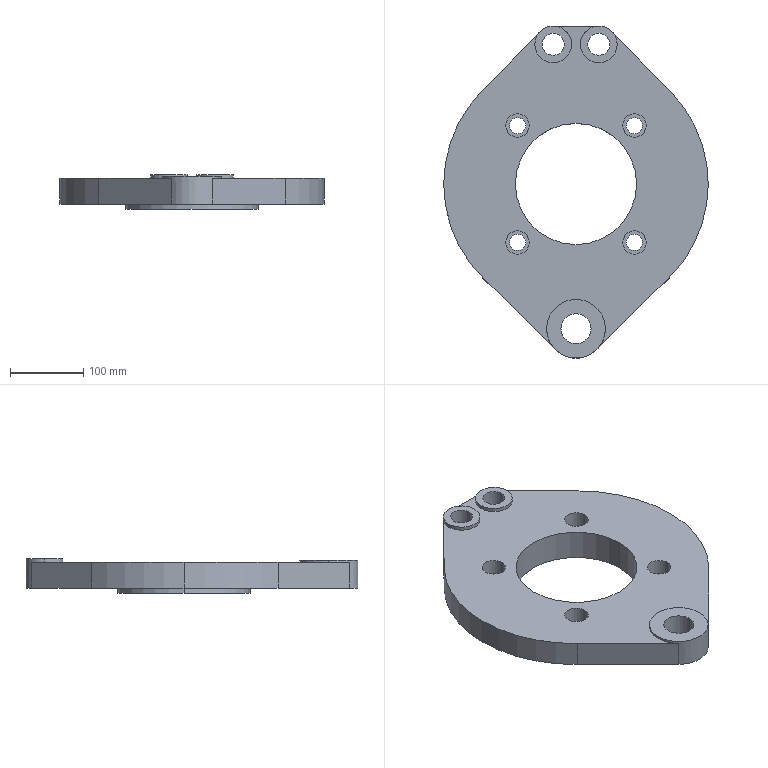Part | SolidWorks | features Boss 3, Cut 2, CirPattern 1, Extrusion 1, RefAxis 1 | 1 solid | 50 faces | box 360 x 452 x 47 mm | volume 3099726 mm3 | cylinder 35 | plane 15 | commonest cylinder face diameters 22 x8 32 x8 30 x4 50 x4 360 x3 41 x2
STEP:
#1=CARTESIAN_POINT('',(-90.,0.,-7.));
#2=VERTEX_POINT('',#1);
#3=CARTESIAN_POINT('',(90.,0.,-7.));
#4=VERTEX_POINT('',#3);
#5=CARTESIAN_POINT('',(0.,0.,-7.));
#6=DIRECTION('',(0.,0.,-1.));
#7=DIRECTION('',(-1.,0.,0.));
#8=AXIS2_PLACEMENT_3D('',#5,#6,#7);
#9=CIRCLE('',#8,90.);
#10=EDGE_CURVE('',#2,#4,#9,.T.);
#11=ORIENTED_EDGE('',*,*,#10,.F.);
#12=CARTESIAN_POINT('',(-90.,0.,0.));
#13=VERTEX_POINT('',#12);
#14=CARTESIAN_POINT('',(-90.,0.,-7.));
#15=DIRECTION('',(0.,0.,1.));
#16=VECTOR('',#15,1000.);
#17=LINE('',#14,#16);
#18=EDGE_CURVE('',#2,#13,#17,.T.);
#19=ORIENTED_EDGE('',*,*,#18,.T.);
#20=CARTESIAN_POINT('',(90.,0.,0.));
#21=VERTEX_POINT('',#20);
#22=CARTESIAN_POINT('',(0.,0.,0.));
#23=DIRECTION('',(0.,0.,-1.));
#24=DIRECTION('',(1.,0.,0.));
#25=AXIS2_PLACEMENT_3D('',#22,#23,#24);
#26=CIRCLE('',#25,90.);
#27=EDGE_CURVE('',#13,#21,#26,.T.);
#28=ORIENTED_EDGE('',*,*,#27,.T.);
#29=CARTESIAN_POINT('',(90.,0.,-7.));
#30=DIRECTION('',(0.,0.,1.));
#31=VECTOR('',#30,1000.);
#32=LINE('',#29,#31);
#33=EDGE_CURVE('',#4,#21,#32,.T.);
#34=ORIENTED_EDGE('',*,*,#33,.F.);
#35=EDGE_LOOP('',(#11,#19,#28,#34));
#36=FACE_OUTER_BOUND('',#35,.T.);
#37=CARTESIAN_POINT('',(0.,0.,-7.));
#38=DIRECTION('',(0.,0.,1.));
#39=DIRECTION('',(1.,0.,0.));
#40=AXIS2_PLACEMENT_3D('',#37,#38,#39);
#41=CYLINDRICAL_SURFACE('',#40,90.);
#42=ADVANCED_FACE('',(#36),#41,.T.);
#43=CARTESIAN_POINT('',(-95.55,-79.55,13.));
#44=VERTEX_POINT('',#43);
#45=CARTESIAN_POINT('',(-63.55,-79.55,13.));
#46=VERTEX_POINT('',#45);
#47=CARTESIAN_POINT('',(-79.55,-79.55,13.));
#48=DIRECTION('',(0.,0.,1.));
#49=DIRECTION('',(0.,1.,0.));
#50=AXIS2_PLACEMENT_3D('',#47,#48,#49);
#51=CIRCLE('',#50,16.);
#52=EDGE_CURVE('',#44,#46,#51,.T.);
#53=ORIENTED_EDGE('',*,*,#52,.F.);
#54=CARTESIAN_POINT('',(-95.55,-79.55,35.));
#55=VERTEX_POINT('',#54);
#56=CARTESIAN_POINT('',(-95.55,-79.55,13.));
#57=DIRECTION('',(0.,0.,1.));
#58=VECTOR('',#57,1000.);
#59=LINE('',#56,#58);
#60=EDGE_CURVE('',#44,#55,#59,.T.);
#61=ORIENTED_EDGE('',*,*,#60,.T.);
#62=CARTESIAN_POINT('',(-63.55,-79.55,35.));
#63=VERTEX_POINT('',#62);
#64=CARTESIAN_POINT('',(-79.55,-79.55,35.));
#65=DIRECTION('',(0.,0.,1.));
#66=DIRECTION('',(0.,1.,0.));
#67=AXIS2_PLACEMENT_3D('',#64,#65,#66);
#68=CIRCLE('',#67,16.);
#69=EDGE_CURVE('',#55,#63,#68,.T.);
#70=ORIENTED_EDGE('',*,*,#69,.T.);
#71=CARTESIAN_POINT('',(-63.55,-79.55,13.));
#72=DIRECTION('',(0.,0.,1.));
#73=VECTOR('',#72,1000.);
#74=LINE('',#71,#73);
#75=EDGE_CURVE('',#46,#63,#74,.T.);
#76=ORIENTED_EDGE('',*,*,#75,.F.);
#77=EDGE_LOOP('',(#53,#61,#70,#76));
#78=FACE_OUTER_BOUND('',#77,.T.);
#79=CARTESIAN_POINT('',(-79.55,-79.55,13.));
#80=DIRECTION('',(0.,0.,1.));
#81=DIRECTION('',(1.,0.,0.));
#82=AXIS2_PLACEMENT_3D('',#79,#80,#81);
#83=CYLINDRICAL_SURFACE('',#82,16.);
#84=ADVANCED_FACE('',(#78),#83,.F.);
#85=CARTESIAN_POINT('',(63.55,-79.55,13.));
#86=VERTEX_POINT('',#85);
#87=CARTESIAN_POINT('',(95.55,-79.55,13.));
#88=VERTEX_POINT('',#87);
#89=CARTESIAN_POINT('',(79.55,-79.55,13.));
#90=DIRECTION('',(0.,0.,1.));
#91=DIRECTION('',(-1.,0.,0.));
#92=AXIS2_PLACEMENT_3D('',#89,#90,#91);
#93=CIRCLE('',#92,16.);
#94=EDGE_CURVE('',#86,#88,#93,.T.);
#95=ORIENTED_EDGE('',*,*,#94,.F.);
#96=CARTESIAN_POINT('',(63.55,-79.55,35.));
#97=VERTEX_POINT('',#96);
#98=CARTESIAN_POINT('',(63.55,-79.55,13.));
#99=DIRECTION('',(0.,0.,1.));
#100=VECTOR('',#99,1000.);
#101=LINE('',#98,#100);
#102=EDGE_CURVE('',#86,#97,#101,.T.);
#103=ORIENTED_EDGE('',*,*,#102,.T.);
#104=CARTESIAN_POINT('',(95.55,-79.55,35.));
#105=VERTEX_POINT('',#104);
#106=CARTESIAN_POINT('',(79.55,-79.55,35.));
#107=DIRECTION('',(0.,0.,1.));
#108=DIRECTION('',(-1.,0.,0.));
#109=AXIS2_PLACEMENT_3D('',#106,#107,#108);
#110=CIRCLE('',#109,16.);
#111=EDGE_CURVE('',#97,#105,#110,.T.);
#112=ORIENTED_EDGE('',*,*,#111,.T.);
#113=CARTESIAN_POINT('',(95.55,-79.55,13.));
#114=DIRECTION('',(0.,0.,1.));
#115=VECTOR('',#114,1000.);
#116=LINE('',#113,#115);
#117=EDGE_CURVE('',#88,#105,#116,.T.);
#118=ORIENTED_EDGE('',*,*,#117,.F.);
#119=EDGE_LOOP('',(#95,#103,#112,#118));
#120=FACE_OUTER_BOUND('',#119,.T.);
#121=CARTESIAN_POINT('',(79.55,-79.55,13.));
#122=DIRECTION('',(0.,0.,1.));
#123=DIRECTION('',(1.,0.,0.));
#124=AXIS2_PLACEMENT_3D('',#121,#122,#123);
#125=CYLINDRICAL_SURFACE('',#124,16.);
#126=ADVANCED_FACE('',(#120),#125,.F.);
#127=CARTESIAN_POINT('',(63.55,79.55,13.));
#128=VERTEX_POINT('',#127);
#129=CARTESIAN_POINT('',(95.55,79.55,13.));
#130=VERTEX_POINT('',#129);
#131=CARTESIAN_POINT('',(79.55,79.55,13.));
#132=DIRECTION('',(0.,0.,1.));
#133=DIRECTION('',(0.,-1.,0.));
#134=AXIS2_PLACEMENT_3D('',#131,#132,#133);
#135=CIRCLE('',#134,16.);
#136=EDGE_CURVE('',#128,#130,#135,.T.);
#137=ORIENTED_EDGE('',*,*,#136,.F.);
#138=CARTESIAN_POINT('',(63.55,79.55,35.));
#139=VERTEX_POINT('',#138);
#140=CARTESIAN_POINT('',(63.55,79.55,13.));
#141=DIRECTION('',(0.,0.,1.));
#142=VECTOR('',#141,1000.);
#143=LINE('',#140,#142);
#144=EDGE_CURVE('',#128,#139,#143,.T.);
#145=ORIENTED_EDGE('',*,*,#144,.T.);
#146=CARTESIAN_POINT('',(95.55,79.55,35.));
#147=VERTEX_POINT('',#146);
#148=CARTESIAN_POINT('',(79.55,79.55,35.));
#149=DIRECTION('',(0.,0.,1.));
#150=DIRECTION('',(0.,-1.,0.));
#151=AXIS2_PLACEMENT_3D('',#148,#149,#150);
#152=CIRCLE('',#151,16.);
#153=EDGE_CURVE('',#139,#147,#152,.T.);
#154=ORIENTED_EDGE('',*,*,#153,.T.);
#155=CARTESIAN_POINT('',(95.55,79.55,13.));
#156=DIRECTION('',(0.,0.,1.));
#157=VECTOR('',#156,1000.);
#158=LINE('',#155,#157);
#159=EDGE_CURVE('',#130,#147,#158,.T.);
#160=ORIENTED_EDGE('',*,*,#159,.F.);
#161=EDGE_LOOP('',(#137,#145,#154,#160));
#162=FACE_OUTER_BOUND('',#161,.T.);
#163=CARTESIAN_POINT('',(79.55,79.55,13.));
#164=DIRECTION('',(0.,0.,1.));
#165=DIRECTION('',(1.,0.,0.));
#166=AXIS2_PLACEMENT_3D('',#163,#164,#165);
#167=CYLINDRICAL_SURFACE('',#166,16.);
#168=ADVANCED_FACE('',(#162),#167,.F.);
#169=CARTESIAN_POINT('',(-95.55,79.55,13.));
#170=VERTEX_POINT('',#169);
#171=CARTESIAN_POINT('',(-63.55,79.55,13.));
#172=VERTEX_POINT('',#171);
#173=CARTESIAN_POINT('',(-79.55,79.55,13.));
#174=DIRECTION('',(0.,0.,1.));
#175=DIRECTION('',(1.,0.,0.));
#176=AXIS2_PLACEMENT_3D('',#173,#174,#175);
#177=CIRCLE('',#176,16.);
#178=EDGE_CURVE('',#170,#172,#177,.T.);
#179=ORIENTED_EDGE('',*,*,#178,.F.);
#180=CARTESIAN_POINT('',(-95.55,79.55,35.));
#181=VERTEX_POINT('',#180);
#182=CARTESIAN_POINT('',(-95.55,79.55,13.));
#183=DIRECTION('',(0.,0.,1.));
#184=VECTOR('',#183,1000.);
#185=LINE('',#182,#184);
#186=EDGE_CURVE('',#170,#181,#185,.T.);
#187=ORIENTED_EDGE('',*,*,#186,.T.);
#188=CARTESIAN_POINT('',(-63.55,79.55,35.));
#189=VERTEX_POINT('',#188);
#190=CARTESIAN_POINT('',(-79.55,79.55,35.));
#191=DIRECTION('',(0.,0.,1.));
#192=DIRECTION('',(1.,0.,0.));
#193=AXIS2_PLACEMENT_3D('',#190,#191,#192);
#194=CIRCLE('',#193,16.);
#195=EDGE_CURVE('',#181,#189,#194,.T.);
#196=ORIENTED_EDGE('',*,*,#195,.T.);
#197=CARTESIAN_POINT('',(-63.55,79.55,13.));
#198=DIRECTION('',(0.,0.,1.));
#199=VECTOR('',#198,1000.);
#200=LINE('',#197,#199);
#201=EDGE_CURVE('',#172,#189,#200,.T.);
#202=ORIENTED_EDGE('',*,*,#201,.F.);
#203=EDGE_LOOP('',(#179,#187,#196,#202));
#204=FACE_OUTER_BOUND('',#203,.T.);
#205=CARTESIAN_POINT('',(-79.55,79.55,13.));
#206=DIRECTION('',(0.,0.,1.));
#207=DIRECTION('',(1.,0.,0.));
#208=AXIS2_PLACEMENT_3D('',#205,#206,#207);
#209=CYLINDRICAL_SURFACE('',#208,16.);
#210=ADVANCED_FACE('',(#204),#209,.F.);
#211=CARTESIAN_POINT('',(-20.5,-197.,38.));
#212=VERTEX_POINT('',#211);
#213=CARTESIAN_POINT('',(20.5,-197.,38.));
#214=VERTEX_POINT('',#213);
#215=CARTESIAN_POINT('',(0.,-197.,38.));
#216=DIRECTION('',(0.,0.,1.));
#217=DIRECTION('',(1.,0.,0.));
#218=AXIS2_PLACEMENT_3D('',#215,#216,#217);
#219=CIRCLE('',#218,20.5);
#220=EDGE_CURVE('',#212,#214,#219,.T.);
#221=ORIENTED_EDGE('',*,*,#220,.T.);
#222=CARTESIAN_POINT('',(20.5,-197.,0.));
#223=VERTEX_POINT('',#222);
#224=CARTESIAN_POINT('',(20.5,-197.,35.));
#225=DIRECTION('',(0.,0.,-1.));
#226=VECTOR('',#225,1000.);
#227=LINE('',#224,#226);
#228=EDGE_CURVE('',#214,#223,#227,.T.);
#229=ORIENTED_EDGE('',*,*,#228,.T.);
#230=CARTESIAN_POINT('',(-20.5,-197.,0.));
#231=VERTEX_POINT('',#230);
#232=CARTESIAN_POINT('',(0.,-197.,0.));
#233=DIRECTION('',(0.,0.,1.));
#234=DIRECTION('',(1.,0.,0.));
#235=AXIS2_PLACEMENT_3D('',#232,#233,#234);
#236=CIRCLE('',#235,20.5);
#237=EDGE_CURVE('',#231,#223,#236,.T.);
#238=ORIENTED_EDGE('',*,*,#237,.F.);
#239=CARTESIAN_POINT('',(-20.5,-197.,35.));
#240=DIRECTION('',(0.,0.,-1.));
#241=VECTOR('',#240,1000.);
#242=LINE('',#239,#241);
#243=EDGE_CURVE('',#212,#231,#242,.T.);
#244=ORIENTED_EDGE('',*,*,#243,.F.);
#245=EDGE_LOOP('',(#221,#229,#238,#244));
#246=FACE_OUTER_BOUND('',#245,.T.);
#247=CARTESIAN_POINT('',(0.,-197.,35.));
#248=DIRECTION('',(0.,0.,-1.));
#249=DIRECTION('',(-1.,0.,0.));
#250=AXIS2_PLACEMENT_3D('',#247,#248,#249);
#251=CYLINDRICAL_SURFACE('',#250,20.5);
#252=ADVANCED_FACE('',(#246),#251,.F.);
#253=CARTESIAN_POINT('',(16.,190.,40.));
#254=VERTEX_POINT('',#253);
#255=CARTESIAN_POINT('',(46.,190.,40.));
#256=VERTEX_POINT('',#255);
#257=CARTESIAN_POINT('',(31.,190.,40.));
#258=DIRECTION('',(0.,0.,1.));
#259=DIRECTION('',(1.,0.,0.));
#260=AXIS2_PLACEMENT_3D('',#257,#258,#259);
#261=CIRCLE('',#260,15.);
#262=EDGE_CURVE('',#254,#256,#261,.T.);
#263=ORIENTED_EDGE('',*,*,#262,.T.);
#264=CARTESIAN_POINT('',(46.,190.,0.));
#265=VERTEX_POINT('',#264);
#266=CARTESIAN_POINT('',(46.,190.,35.));
#267=DIRECTION('',(0.,0.,-1.));
#268=VECTOR('',#267,1000.);
#269=LINE('',#266,#268);
#270=EDGE_CURVE('',#256,#265,#269,.T.);
#271=ORIENTED_EDGE('',*,*,#270,.T.);
#272=CARTESIAN_POINT('',(16.,190.,0.));
#273=VERTEX_POINT('',#272);
#274=CARTESIAN_POINT('',(31.,190.,0.));
#275=DIRECTION('',(0.,0.,1.));
#276=DIRECTION('',(1.,0.,0.));
#277=AXIS2_PLACEMENT_3D('',#274,#275,#276);
#278=CIRCLE('',#277,15.);
#279=EDGE_CURVE('',#273,#265,#278,.T.);
#280=ORIENTED_EDGE('',*,*,#279,.F.);
#281=CARTESIAN_POINT('',(16.,190.,35.));
#282=DIRECTION('',(0.,0.,-1.));
#283=VECTOR('',#282,1000.);
#284=LINE('',#281,#283);
#285=EDGE_CURVE('',#254,#273,#284,.T.);
#286=ORIENTED_EDGE('',*,*,#285,.F.);
#287=EDGE_LOOP('',(#263,#271,#280,#286));
#288=FACE_OUTER_BOUND('',#287,.T.);
#289=CARTESIAN_POINT('',(31.,190.,35.));
#290=DIRECTION('',(0.,0.,-1.));
#291=DIRECTION('',(-1.,0.,0.));
#292=AXIS2_PLACEMENT_3D('',#289,#290,#291);
#293=CYLINDRICAL_SURFACE('',#292,15.);
#294=ADVANCED_FACE('',(#288),#293,.F.);
#295=CARTESIAN_POINT('',(-46.,190.,40.));
#296=VERTEX_POINT('',#295);
#297=CARTESIAN_POINT('',(-16.,190.,40.));
#298=VERTEX_POINT('',#297);
#299=CARTESIAN_POINT('',(-31.,190.,40.));
#300=DIRECTION('',(0.,0.,1.));
#301=DIRECTION('',(1.,0.,0.));
#302=AXIS2_PLACEMENT_3D('',#299,#300,#301);
#303=CIRCLE('',#302,15.);
#304=EDGE_CURVE('',#296,#298,#303,.T.);
#305=ORIENTED_EDGE('',*,*,#304,.T.);
#306=CARTESIAN_POINT('',(-16.,190.,0.));
#307=VERTEX_POINT('',#306);
#308=CARTESIAN_POINT('',(-16.,190.,35.));
#309=DIRECTION('',(0.,0.,-1.));
#310=VECTOR('',#309,1000.);
#311=LINE('',#308,#310);
#312=EDGE_CURVE('',#298,#307,#311,.T.);
#313=ORIENTED_EDGE('',*,*,#312,.T.);
#314=CARTESIAN_POINT('',(-46.,190.,0.));
#315=VERTEX_POINT('',#314);
#316=CARTESIAN_POINT('',(-31.,190.,0.));
#317=DIRECTION('',(0.,0.,1.));
#318=DIRECTION('',(1.,0.,0.));
#319=AXIS2_PLACEMENT_3D('',#316,#317,#318);
#320=CIRCLE('',#319,15.);
#321=EDGE_CURVE('',#315,#307,#320,.T.);
#322=ORIENTED_EDGE('',*,*,#321,.F.);
#323=CARTESIAN_POINT('',(-46.,190.,35.));
#324=DIRECTION('',(0.,0.,-1.));
#325=VECTOR('',#324,1000.);
#326=LINE('',#323,#325);
#327=EDGE_CURVE('',#296,#315,#326,.T.);
#328=ORIENTED_EDGE('',*,*,#327,.F.);
#329=EDGE_LOOP('',(#305,#313,#322,#328));
#330=FACE_OUTER_BOUND('',#329,.T.);
#331=CARTESIAN_POINT('',(-31.,190.,35.));
#332=DIRECTION('',(0.,0.,-1.));
#333=DIRECTION('',(-1.,0.,0.));
#334=AXIS2_PLACEMENT_3D('',#331,#332,#333);
#335=CYLINDRICAL_SURFACE('',#334,15.);
#336=ADVANCED_FACE('',(#330),#335,.F.);
#337=CARTESIAN_POINT('',(-82.5,0.,35.));
#338=VERTEX_POINT('',#337);
#339=CARTESIAN_POINT('',(82.5,0.,35.));
#340=VERTEX_POINT('',#339);
#341=CARTESIAN_POINT('',(0.,0.,35.));
#342=DIRECTION('',(0.,0.,1.));
#343=DIRECTION('',(1.,0.,0.));
#344=AXIS2_PLACEMENT_3D('',#341,#342,#343);
#345=CIRCLE('',#344,82.5);
#346=EDGE_CURVE('',#338,#340,#345,.T.);
#347=ORIENTED_EDGE('',*,*,#346,.T.);
#348=CARTESIAN_POINT('',(82.5,0.,-7.));
#349=VERTEX_POINT('',#348);
#350=CARTESIAN_POINT('',(82.5,0.,35.));
#351=DIRECTION('',(0.,0.,-1.));
#352=VECTOR('',#351,1000.);
#353=LINE('',#350,#352);
#354=EDGE_CURVE('',#340,#349,#353,.T.);
#355=ORIENTED_EDGE('',*,*,#354,.T.);
#356=CARTESIAN_POINT('',(-82.5,0.,-7.));
#357=VERTEX_POINT('',#356);
#358=CARTESIAN_POINT('',(0.,0.,-7.));
#359=DIRECTION('',(0.,0.,-1.));
#360=DIRECTION('',(-1.,0.,0.));
#361=AXIS2_PLACEMENT_3D('',#358,#359,#360);
#362=CIRCLE('',#361,82.5);
#363=EDGE_CURVE('',#349,#357,#362,.T.);
#364=ORIENTED_EDGE('',*,*,#363,.T.);
#365=CARTESIAN_POINT('',(-82.5,0.,35.));
#366=DIRECTION('',(0.,0.,-1.));
#367=VECTOR('',#366,1000.);
#368=LINE('',#365,#367);
#369=EDGE_CURVE('',#338,#357,#368,.T.);
#370=ORIENTED_EDGE('',*,*,#369,.F.);
#371=EDGE_LOOP('',(#347,#355,#364,#370));
#372=FACE_OUTER_BOUND('',#371,.T.);
#373=CARTESIAN_POINT('',(0.,0.,35.));
#374=DIRECTION('',(0.,0.,-1.));
#375=DIRECTION('',(-1.,0.,0.));
#376=AXIS2_PLACEMENT_3D('',#373,#374,#375);
#377=CYLINDRICAL_SURFACE('',#376,82.5);
#378=ADVANCED_FACE('',(#372),#377,.F.);
#379=CARTESIAN_POINT('',(-180.,0.,35.));
#380=VERTEX_POINT('',#379);
#381=CARTESIAN_POINT('',(-126.636,-127.919,35.));
#382=VERTEX_POINT('',#381);
#383=CARTESIAN_POINT('',(0.,0.,35.));
#384=DIRECTION('',(0.,0.,1.));
#385=DIRECTION('',(1.,0.,0.));
#386=AXIS2_PLACEMENT_3D('',#383,#384,#385);
#387=CIRCLE('',#386,180.);
#388=EDGE_CURVE('',#380,#382,#387,.T.);
#389=ORIENTED_EDGE('',*,*,#388,.F.);
#390=CARTESIAN_POINT('',(-180.,0.,0.));
#391=VERTEX_POINT('',#390);
#392=CARTESIAN_POINT('',(-180.,0.,35.));
#393=DIRECTION('',(0.,0.,-1.));
#394=VECTOR('',#393,1000.);
#395=LINE('',#392,#394);
#396=EDGE_CURVE('',#380,#391,#395,.T.);
#397=ORIENTED_EDGE('',*,*,#396,.T.);
#398=CARTESIAN_POINT('',(-126.636,-127.919,0.));
#399=VERTEX_POINT('',#398);
#400=CARTESIAN_POINT('',(0.,0.,0.));
#401=DIRECTION('',(0.,0.,1.));
#402=DIRECTION('',(1.,0.,0.));
#403=AXIS2_PLACEMENT_3D('',#400,#401,#402);
#404=CIRCLE('',#403,180.);
#405=EDGE_CURVE('',#391,#399,#404,.T.);
#406=ORIENTED_EDGE('',*,*,#405,.T.);
#407=CARTESIAN_POINT('',(-126.636,-127.919,35.));
#408=DIRECTION('',(0.,0.,-1.));
#409=VECTOR('',#408,1000.);
#410=LINE('',#407,#409);
#411=EDGE_CURVE('',#382,#399,#410,.T.);
#412=ORIENTED_EDGE('',*,*,#411,.F.);
#413=EDGE_LOOP('',(#389,#397,#406,#412));
#414=FACE_OUTER_BOUND('',#413,.T.);
#415=CARTESIAN_POINT('',(0.,0.,35.));
#416=DIRECTION('',(0.,0.,-1.));
#417=DIRECTION('',(-1.,0.,0.));
#418=AXIS2_PLACEMENT_3D('',#415,#416,#417);
#419=CYLINDRICAL_SURFACE('',#418,180.);
#420=ADVANCED_FACE('',(#414),#419,.T.);
#421=CARTESIAN_POINT('',(-6.,190.,40.));
#422=VERTEX_POINT('',#421);
#423=CARTESIAN_POINT('',(-56.,190.,40.));
#424=VERTEX_POINT('',#423);
#425=CARTESIAN_POINT('',(-31.,190.,40.));
#426=DIRECTION('',(0.,0.,1.));
#427=DIRECTION('',(1.,0.,0.));
#428=AXIS2_PLACEMENT_3D('',#425,#426,#427);
#429=CIRCLE('',#428,25.);
#430=EDGE_CURVE('',#422,#424,#429,.T.);
#431=ORIENTED_EDGE('',*,*,#430,.F.);
#432=CARTESIAN_POINT('',(-6.,190.,35.));
#433=VERTEX_POINT('',#432);
#434=CARTESIAN_POINT('',(-6.,190.,35.));
#435=DIRECTION('',(0.,0.,-1.));
#436=VECTOR('',#435,1000.);
#437=LINE('',#434,#436);
#438=EDGE_CURVE('',#422,#433,#437,.T.);
#439=ORIENTED_EDGE('',*,*,#438,.T.);
#440=CARTESIAN_POINT('',(-31.,215.,35.));
#441=VERTEX_POINT('',#440);
#442=CARTESIAN_POINT('',(-31.,190.,35.));
#443=DIRECTION('',(0.,0.,1.));
#444=DIRECTION('',(1.,0.,0.));
#445=AXIS2_PLACEMENT_3D('',#442,#443,#444);
#446=CIRCLE('',#445,25.);
#447=EDGE_CURVE('',#433,#441,#446,.T.);
#448=ORIENTED_EDGE('',*,*,#447,.T.);
#449=CARTESIAN_POINT('',(-31.,215.,0.));
#450=VERTEX_POINT('',#449);
#451=CARTESIAN_POINT('',(-31.,215.,35.));
#452=DIRECTION('',(0.,0.,-1.));
#453=VECTOR('',#452,1000.);
#454=LINE('',#451,#453);
#455=EDGE_CURVE('',#441,#450,#454,.T.);
#456=ORIENTED_EDGE('',*,*,#455,.T.);
#457=CARTESIAN_POINT('',(-48.875,207.478,0.));
#458=VERTEX_POINT('',#457);
#459=CARTESIAN_POINT('',(-31.,190.,0.));
#460=DIRECTION('',(0.,0.,1.));
#461=DIRECTION('',(1.,0.,0.));
#462=AXIS2_PLACEMENT_3D('',#459,#460,#461);
#463=CIRCLE('',#462,25.);
#464=EDGE_CURVE('',#450,#458,#463,.T.);
#465=ORIENTED_EDGE('',*,*,#464,.T.);
#466=CARTESIAN_POINT('',(-48.875,207.478,35.));
#467=VERTEX_POINT('',#466);
#468=CARTESIAN_POINT('',(-48.875,207.478,35.));
#469=DIRECTION('',(0.,0.,-1.));
#470=VECTOR('',#469,1000.);
#471=LINE('',#468,#470);
#472=EDGE_CURVE('',#467,#458,#471,.T.);
#473=ORIENTED_EDGE('',*,*,#472,.F.);
#474=CARTESIAN_POINT('',(-56.,190.,35.));
#475=VERTEX_POINT('',#474);
#476=CARTESIAN_POINT('',(-31.,190.,35.));
#477=DIRECTION('',(0.,0.,1.));
#478=DIRECTION('',(1.,0.,0.));
#479=AXIS2_PLACEMENT_3D('',#476,#477,#478);
#480=CIRCLE('',#479,25.);
#481=EDGE_CURVE('',#467,#475,#480,.T.);
#482=ORIENTED_EDGE('',*,*,#481,.T.);
#483=CARTESIAN_POINT('',(-56.,190.,35.));
#484=DIRECTION('',(0.,0.,-1.));
#485=VECTOR('',#484,1000.);
#486=LINE('',#483,#485);
#487=EDGE_CURVE('',#424,#475,#486,.T.);
#488=ORIENTED_EDGE('',*,*,#487,.F.);
#489=EDGE_LOOP('',(#431,#439,#448,#456,#465,#473,#482,#488));
#490=FACE_OUTER_BOUND('',#489,.T.);
#491=CARTESIAN_POINT('',(-31.,190.,35.));
#492=DIRECTION('',(0.,0.,-1.));
#493=DIRECTION('',(-1.,0.,0.));
#494=AXIS2_PLACEMENT_3D('',#491,#492,#493);
#495=CYLINDRICAL_SURFACE('',#494,25.);
#496=ADVANCED_FACE('',(#490),#495,.T.);
#497=CARTESIAN_POINT('',(56.,190.,40.));
#498=VERTEX_POINT('',#497);
#499=CARTESIAN_POINT('',(6.,190.,40.));
#500=VERTEX_POINT('',#499);
#501=CARTESIAN_POINT('',(31.,190.,40.));
#502=DIRECTION('',(0.,0.,1.));
#503=DIRECTION('',(1.,0.,0.));
#504=AXIS2_PLACEMENT_3D('',#501,#502,#503);
#505=CIRCLE('',#504,25.);
#506=EDGE_CURVE('',#498,#500,#505,.T.);
#507=ORIENTED_EDGE('',*,*,#506,.F.);
#508=CARTESIAN_POINT('',(56.,190.,35.));
#509=VERTEX_POINT('',#508);
#510=CARTESIAN_POINT('',(56.,190.,35.));
#511=DIRECTION('',(0.,0.,-1.));
#512=VECTOR('',#511,1000.);
#513=LINE('',#510,#512);
#514=EDGE_CURVE('',#498,#509,#513,.T.);
#515=ORIENTED_EDGE('',*,*,#514,.T.);
#516=CARTESIAN_POINT('',(48.875,207.478,35.));
#517=VERTEX_POINT('',#516);
#518=CARTESIAN_POINT('',(31.,190.,35.));
#519=DIRECTION('',(0.,0.,1.));
#520=DIRECTION('',(1.,0.,0.));
#521=AXIS2_PLACEMENT_3D('',#518,#519,#520);
#522=CIRCLE('',#521,25.);
#523=EDGE_CURVE('',#509,#517,#522,.T.);
#524=ORIENTED_EDGE('',*,*,#523,.T.);
#525=CARTESIAN_POINT('',(48.875,207.478,0.));
#526=VERTEX_POINT('',#525);
#527=CARTESIAN_POINT('',(48.875,207.478,35.));
#528=DIRECTION('',(0.,0.,-1.));
#529=VECTOR('',#528,1000.);
#530=LINE('',#527,#529);
#531=EDGE_CURVE('',#517,#526,#530,.T.);
#532=ORIENTED_EDGE('',*,*,#531,.T.);
#533=CARTESIAN_POINT('',(31.,215.,0.));
#534=VERTEX_POINT('',#533);
#535=CARTESIAN_POINT('',(31.,190.,0.));
#536=DIRECTION('',(0.,0.,1.));
#537=DIRECTION('',(1.,0.,0.));
#538=AXIS2_PLACEMENT_3D('',#535,#536,#537);
#539=CIRCLE('',#538,25.);
#540=EDGE_CURVE('',#526,#534,#539,.T.);
#541=ORIENTED_EDGE('',*,*,#540,.T.);
#542=CARTESIAN_POINT('',(31.,215.,35.));
#543=VERTEX_POINT('',#542);
#544=CARTESIAN_POINT('',(31.,215.,35.));
#545=DIRECTION('',(0.,0.,-1.));
#546=VECTOR('',#545,1000.);
#547=LINE('',#544,#546);
#548=EDGE_CURVE('',#543,#534,#547,.T.);
#549=ORIENTED_EDGE('',*,*,#548,.F.);
#550=CARTESIAN_POINT('',(6.,190.,35.));
#551=VERTEX_POINT('',#550);
#552=CARTESIAN_POINT('',(31.,190.,35.));
#553=DIRECTION('',(0.,0.,1.));
#554=DIRECTION('',(1.,0.,0.));
#555=AXIS2_PLACEMENT_3D('',#552,#553,#554);
#556=CIRCLE('',#555,25.);
#557=EDGE_CURVE('',#543,#551,#556,.T.);
#558=ORIENTED_EDGE('',*,*,#557,.T.);
#559=CARTESIAN_POINT('',(6.,190.,35.));
#560=DIRECTION('',(0.,0.,-1.));
#561=VECTOR('',#560,1000.);
#562=LINE('',#559,#561);
#563=EDGE_CURVE('',#500,#551,#562,.T.);
#564=ORIENTED_EDGE('',*,*,#563,.F.);
#565=EDGE_LOOP('',(#507,#515,#524,#532,#541,#549,#558,#564));
#566=FACE_OUTER_BOUND('',#565,.T.);
#567=CARTESIAN_POINT('',(31.,190.,35.));
#568=DIRECTION('',(0.,0.,-1.));
#569=DIRECTION('',(-1.,0.,0.));
#570=AXIS2_PLACEMENT_3D('',#567,#568,#569);
#571=CYLINDRICAL_SURFACE('',#570,25.);
#572=ADVANCED_FACE('',(#566),#571,.T.);
#573=CARTESIAN_POINT('',(40.,-197.,38.));
#574=VERTEX_POINT('',#573);
#575=CARTESIAN_POINT('',(-40.,-197.,38.));
#576=VERTEX_POINT('',#575);
#577=CARTESIAN_POINT('',(0.,-197.,38.));
#578=DIRECTION('',(0.,0.,1.));
#579=DIRECTION('',(1.,0.,0.));
#580=AXIS2_PLACEMENT_3D('',#577,#578,#579);
#581=CIRCLE('',#580,40.);
#582=EDGE_CURVE('',#574,#576,#581,.T.);
#583=ORIENTED_EDGE('',*,*,#582,.F.);
#584=CARTESIAN_POINT('',(40.,-197.,35.));
#585=VERTEX_POINT('',#584);
#586=CARTESIAN_POINT('',(40.,-197.,35.));
#587=DIRECTION('',(0.,0.,-1.));
#588=VECTOR('',#587,1000.);
#589=LINE('',#586,#588);
#590=EDGE_CURVE('',#574,#585,#589,.T.);
#591=ORIENTED_EDGE('',*,*,#590,.T.);
#592=CARTESIAN_POINT('',(-40.,-197.,35.));
#593=VERTEX_POINT('',#592);
#594=CARTESIAN_POINT('',(0.,-197.,35.));
#595=DIRECTION('',(0.,0.,1.));
#596=DIRECTION('',(1.,0.,0.));
#597=AXIS2_PLACEMENT_3D('',#594,#595,#596);
#598=CIRCLE('',#597,40.);
#599=EDGE_CURVE('',#585,#593,#598,.T.);
#600=ORIENTED_EDGE('',*,*,#599,.T.);
#601=CARTESIAN_POINT('',(-40.,-197.,35.));
#602=DIRECTION('',(0.,0.,-1.));
#603=VECTOR('',#602,1000.);
#604=LINE('',#601,#603);
#605=EDGE_CURVE('',#576,#593,#604,.T.);
#606=ORIENTED_EDGE('',*,*,#605,.F.);
#607=EDGE_LOOP('',(#583,#591,#600,#606));
#608=FACE_OUTER_BOUND('',#607,.T.);
#609=CARTESIAN_POINT('',(0.,-197.,35.));
#610=DIRECTION('',(0.,0.,-1.));
#611=DIRECTION('',(-1.,0.,0.));
#612=AXIS2_PLACEMENT_3D('',#609,#610,#611);
#613=CYLINDRICAL_SURFACE('',#612,40.);
#614=ADVANCED_FACE('',(#608),#613,.T.);
#615=CARTESIAN_POINT('',(-68.55,79.55,0.));
#616=VERTEX_POINT('',#615);
#617=CARTESIAN_POINT('',(-90.55,79.55,0.));
#618=VERTEX_POINT('',#617);
#619=CARTESIAN_POINT('',(-79.55,79.55,0.));
#620=DIRECTION('',(0.,0.,-1.));
#621=DIRECTION('',(1.,0.,0.));
#622=AXIS2_PLACEMENT_3D('',#619,#620,#621);
#623=CIRCLE('',#622,11.);
#624=EDGE_CURVE('',#616,#618,#623,.T.);
#625=ORIENTED_EDGE('',*,*,#624,.T.);
#626=CARTESIAN_POINT('',(-90.55,79.55,13.));
#627=VERTEX_POINT('',#626);
#628=CARTESIAN_POINT('',(-90.55,79.55,-0.001025));
#629=DIRECTION('',(0.,0.,1.));
#630=VECTOR('',#629,1000.);
#631=LINE('',#628,#630);
#632=EDGE_CURVE('',#618,#627,#631,.T.);
#633=ORIENTED_EDGE('',*,*,#632,.T.);
#634=CARTESIAN_POINT('',(-68.55,79.55,13.));
#635=VERTEX_POINT('',#634);
#636=CARTESIAN_POINT('',(-79.55,79.55,13.));
#637=DIRECTION('',(0.,0.,-1.));
#638=DIRECTION('',(1.,0.,0.));
#639=AXIS2_PLACEMENT_3D('',#636,#637,#638);
#640=CIRCLE('',#639,11.);
#641=EDGE_CURVE('',#635,#627,#640,.T.);
#642=ORIENTED_EDGE('',*,*,#641,.F.);
#643=CARTESIAN_POINT('',(-68.55,79.55,-0.001025));
#644=DIRECTION('',(0.,0.,1.));
#645=VECTOR('',#644,1000.);
#646=LINE('',#643,#645);
#647=EDGE_CURVE('',#616,#635,#646,.T.);
#648=ORIENTED_EDGE('',*,*,#647,.F.);
#649=EDGE_LOOP('',(#625,#633,#642,#648));
#650=FACE_OUTER_BOUND('',#649,.T.);
#651=CARTESIAN_POINT('',(-79.55,79.55,-0.001025));
#652=DIRECTION('',(0.,0.,1.));
#653=DIRECTION('',(1.,0.,0.));
#654=AXIS2_PLACEMENT_3D('',#651,#652,#653);
#655=CYLINDRICAL_SURFACE('',#654,11.);
#656=ADVANCED_FACE('',(#650),#655,.F.);
#657=CARTESIAN_POINT('',(90.55,79.55,0.));
#658=VERTEX_POINT('',#657);
#659=CARTESIAN_POINT('',(68.55,79.55,0.));
#660=VERTEX_POINT('',#659);
#661=CARTESIAN_POINT('',(79.55,79.55,0.));
#662=DIRECTION('',(0.,0.,-1.));
#663=DIRECTION('',(1.,0.,0.));
#664=AXIS2_PLACEMENT_3D('',#661,#662,#663);
#665=CIRCLE('',#664,11.);
#666=EDGE_CURVE('',#658,#660,#665,.T.);
#667=ORIENTED_EDGE('',*,*,#666,.T.);
#668=CARTESIAN_POINT('',(68.55,79.55,13.));
#669=VERTEX_POINT('',#668);
#670=CARTESIAN_POINT('',(68.55,79.55,-0.001025));
#671=DIRECTION('',(0.,0.,1.));
#672=VECTOR('',#671,1000.);
#673=LINE('',#670,#672);
#674=EDGE_CURVE('',#660,#669,#673,.T.);
#675=ORIENTED_EDGE('',*,*,#674,.T.);
#676=CARTESIAN_POINT('',(90.55,79.55,13.));
#677=VERTEX_POINT('',#676);
#678=CARTESIAN_POINT('',(79.55,79.55,13.));
#679=DIRECTION('',(0.,0.,-1.));
#680=DIRECTION('',(1.,0.,0.));
#681=AXIS2_PLACEMENT_3D('',#678,#679,#680);
#682=CIRCLE('',#681,11.);
#683=EDGE_CURVE('',#677,#669,#682,.T.);
#684=ORIENTED_EDGE('',*,*,#683,.F.);
#685=CARTESIAN_POINT('',(90.55,79.55,-0.001025));
#686=DIRECTION('',(0.,0.,1.));
#687=VECTOR('',#686,1000.);
#688=LINE('',#685,#687);
#689=EDGE_CURVE('',#658,#677,#688,.T.);
#690=ORIENTED_EDGE('',*,*,#689,.F.);
#691=EDGE_LOOP('',(#667,#675,#684,#690));
#692=FACE_OUTER_BOUND('',#691,.T.);
#693=CARTESIAN_POINT('',(79.55,79.55,-0.001025));
#694=DIRECTION('',(0.,0.,1.));
#695=DIRECTION('',(1.,0.,0.));
#696=AXIS2_PLACEMENT_3D('',#693,#694,#695);
#697=CYLINDRICAL_SURFACE('',#696,11.);
#698=ADVANCED_FACE('',(#692),#697,.F.);
#699=CARTESIAN_POINT('',(90.55,-79.55,0.));
#700=VERTEX_POINT('',#699);
#701=CARTESIAN_POINT('',(68.55,-79.55,0.));
#702=VERTEX_POINT('',#701);
#703=CARTESIAN_POINT('',(79.55,-79.55,0.));
#704=DIRECTION('',(0.,0.,-1.));
#705=DIRECTION('',(1.,0.,0.));
#706=AXIS2_PLACEMENT_3D('',#703,#704,#705);
#707=CIRCLE('',#706,11.);
#708=EDGE_CURVE('',#700,#702,#707,.T.);
#709=ORIENTED_EDGE('',*,*,#708,.T.);
#710=CARTESIAN_POINT('',(68.55,-79.55,13.));
#711=VERTEX_POINT('',#710);
#712=CARTESIAN_POINT('',(68.55,-79.55,-0.001025));
#713=DIRECTION('',(0.,0.,1.));
#714=VECTOR('',#713,1000.);
#715=LINE('',#712,#714);
#716=EDGE_CURVE('',#702,#711,#715,.T.);
#717=ORIENTED_EDGE('',*,*,#716,.T.);
#718=CARTESIAN_POINT('',(90.55,-79.55,13.));
#719=VERTEX_POINT('',#718);
#720=CARTESIAN_POINT('',(79.55,-79.55,13.));
#721=DIRECTION('',(0.,0.,-1.));
#722=DIRECTION('',(1.,0.,0.));
#723=AXIS2_PLACEMENT_3D('',#720,#721,#722);
#724=CIRCLE('',#723,11.);
#725=EDGE_CURVE('',#719,#711,#724,.T.);
#726=ORIENTED_EDGE('',*,*,#725,.F.);
#727=CARTESIAN_POINT('',(90.55,-79.55,-0.001025));
#728=DIRECTION('',(0.,0.,1.));
#729=VECTOR('',#728,1000.);
#730=LINE('',#727,#729);
#731=EDGE_CURVE('',#700,#719,#730,.T.);
#732=ORIENTED_EDGE('',*,*,#731,.F.);
#733=EDGE_LOOP('',(#709,#717,#726,#732));
#734=FACE_OUTER_BOUND('',#733,.T.);
#735=CARTESIAN_POINT('',(79.55,-79.55,-0.001025));
#736=DIRECTION('',(0.,0.,1.));
#737=DIRECTION('',(1.,0.,0.));
#738=AXIS2_PLACEMENT_3D('',#735,#736,#737);
#739=CYLINDRICAL_SURFACE('',#738,11.);
#740=ADVANCED_FACE('',(#734),#739,.F.);
#741=CARTESIAN_POINT('',(-68.55,-79.55,0.));
#742=VERTEX_POINT('',#741);
#743=CARTESIAN_POINT('',(-90.55,-79.55,0.));
#744=VERTEX_POINT('',#743);
#745=CARTESIAN_POINT('',(-79.55,-79.55,0.));
#746=DIRECTION('',(0.,0.,-1.));
#747=DIRECTION('',(1.,0.,0.));
#748=AXIS2_PLACEMENT_3D('',#745,#746,#747);
#749=CIRCLE('',#748,11.);
#750=EDGE_CURVE('',#742,#744,#749,.T.);
#751=ORIENTED_EDGE('',*,*,#750,.T.);
#752=CARTESIAN_POINT('',(-90.55,-79.55,13.));
#753=VERTEX_POINT('',#752);
#754=CARTESIAN_POINT('',(-90.55,-79.55,-0.001025));
#755=DIRECTION('',(0.,0.,1.));
#756=VECTOR('',#755,1000.);
#757=LINE('',#754,#756);
#758=EDGE_CURVE('',#744,#753,#757,.T.);
#759=ORIENTED_EDGE('',*,*,#758,.T.);
#760=CARTESIAN_POINT('',(-68.55,-79.55,13.));
#761=VERTEX_POINT('',#760);
#762=CARTESIAN_POINT('',(-79.55,-79.55,13.));
#763=DIRECTION('',(0.,0.,-1.));
#764=DIRECTION('',(1.,0.,0.));
#765=AXIS2_PLACEMENT_3D('',#762,#763,#764);
#766=CIRCLE('',#765,11.);
#767=EDGE_CURVE('',#761,#753,#766,.T.);
#768=ORIENTED_EDGE('',*,*,#767,.F.);
#769=CARTESIAN_POINT('',(-68.55,-79.55,-0.001025));
#770=DIRECTION('',(0.,0.,1.));
#771=VECTOR('',#770,1000.);
#772=LINE('',#769,#771);
#773=EDGE_CURVE('',#742,#761,#772,.T.);
#774=ORIENTED_EDGE('',*,*,#773,.F.);
#775=EDGE_LOOP('',(#751,#759,#768,#774));
#776=FACE_OUTER_BOUND('',#775,.T.);
#777=CARTESIAN_POINT('',(-79.55,-79.55,-0.001025));
#778=DIRECTION('',(0.,0.,1.));
#779=DIRECTION('',(1.,0.,0.));
#780=AXIS2_PLACEMENT_3D('',#777,#778,#779);
#781=CYLINDRICAL_SURFACE('',#780,11.);
#782=ADVANCED_FACE('',(#776),#781,.F.);
#783=ORIENTED_EDGE('',*,*,#237,.T.);
#784=CARTESIAN_POINT('',(0.,-197.,0.));
#785=DIRECTION('',(0.,0.,1.));
#786=DIRECTION('',(1.,0.,0.));
#787=AXIS2_PLACEMENT_3D('',#784,#785,#786);
#788=CIRCLE('',#787,20.5);
#789=EDGE_CURVE('',#223,#231,#788,.T.);
#790=ORIENTED_EDGE('',*,*,#789,.T.);
#791=EDGE_LOOP('',(#783,#790));
#792=FACE_BOUND('',#791,.T.);
#793=ORIENTED_EDGE('',*,*,#321,.T.);
#794=CARTESIAN_POINT('',(-31.,190.,0.));
#795=DIRECTION('',(0.,0.,1.));
#796=DIRECTION('',(1.,0.,0.));
#797=AXIS2_PLACEMENT_3D('',#794,#795,#796);
#798=CIRCLE('',#797,15.);
#799=EDGE_CURVE('',#307,#315,#798,.T.);
#800=ORIENTED_EDGE('',*,*,#799,.T.);
#801=EDGE_LOOP('',(#793,#800));
#802=FACE_BOUND('',#801,.T.);
#803=CARTESIAN_POINT('',(-28.141,-225.426,0.));
#804=VERTEX_POINT('',#803);
#805=CARTESIAN_POINT('',(28.141,-225.426,0.));
#806=VERTEX_POINT('',#805);
#807=CARTESIAN_POINT('',(0.,-197.,0.));
#808=DIRECTION('',(0.,0.,1.));
#809=DIRECTION('',(1.,0.,0.));
#810=AXIS2_PLACEMENT_3D('',#807,#808,#809);
#811=CIRCLE('',#810,40.);
#812=EDGE_CURVE('',#804,#806,#811,.T.);
#813=ORIENTED_EDGE('',*,*,#812,.F.);
#814=CARTESIAN_POINT('',(-28.141,-225.426,0.));
#815=DIRECTION('',(0.7107,-0.7035,0.));
#816=VECTOR('',#815,1000.);
#817=LINE('',#814,#816);
#818=EDGE_CURVE('',#399,#804,#817,.T.);
#819=ORIENTED_EDGE('',*,*,#818,.F.);
#820=ORIENTED_EDGE('',*,*,#405,.F.);
#821=CARTESIAN_POINT('',(-128.699,125.844,0.));
#822=VERTEX_POINT('',#821);
#823=CARTESIAN_POINT('',(0.,0.,0.));
#824=DIRECTION('',(0.,0.,1.));
#825=DIRECTION('',(1.,0.,0.));
#826=AXIS2_PLACEMENT_3D('',#823,#824,#825);
#827=CIRCLE('',#826,180.);
#828=EDGE_CURVE('',#822,#391,#827,.T.);
#829=ORIENTED_EDGE('',*,*,#828,.F.);
#830=CARTESIAN_POINT('',(-48.875,207.478,0.));
#831=DIRECTION('',(-0.6991,-0.715,0.));
#832=VECTOR('',#831,1000.);
#833=LINE('',#830,#832);
#834=EDGE_CURVE('',#458,#822,#833,.T.);
#835=ORIENTED_EDGE('',*,*,#834,.F.);
#836=ORIENTED_EDGE('',*,*,#464,.F.);
#837=CARTESIAN_POINT('',(-31.,215.,0.));
#838=DIRECTION('',(-1.,0.,0.));
#839=VECTOR('',#838,1000.);
#840=LINE('',#837,#839);
#841=EDGE_CURVE('',#534,#450,#840,.T.);
#842=ORIENTED_EDGE('',*,*,#841,.F.);
#843=ORIENTED_EDGE('',*,*,#540,.F.);
#844=CARTESIAN_POINT('',(128.699,125.844,0.));
#845=VERTEX_POINT('',#844);
#846=CARTESIAN_POINT('',(48.875,207.478,0.));
#847=DIRECTION('',(-0.6991,0.715,0.));
#848=VECTOR('',#847,1000.);
#849=LINE('',#846,#848);
#850=EDGE_CURVE('',#845,#526,#849,.T.);
#851=ORIENTED_EDGE('',*,*,#850,.F.);
#852=CARTESIAN_POINT('',(126.636,-127.919,0.));
#853=VERTEX_POINT('',#852);
#854=CARTESIAN_POINT('',(0.,0.,0.));
#855=DIRECTION('',(0.,0.,1.));
#856=DIRECTION('',(1.,0.,0.));
#857=AXIS2_PLACEMENT_3D('',#854,#855,#856);
#858=CIRCLE('',#857,180.);
#859=EDGE_CURVE('',#853,#845,#858,.T.);
#860=ORIENTED_EDGE('',*,*,#859,.F.);
#861=CARTESIAN_POINT('',(28.141,-225.426,0.));
#862=DIRECTION('',(0.7107,0.7035,0.));
#863=VECTOR('',#862,1000.);
#864=LINE('',#861,#863);
#865=EDGE_CURVE('',#806,#853,#864,.T.);
#866=ORIENTED_EDGE('',*,*,#865,.F.);
#867=EDGE_LOOP('',(#813,#819,#820,#829,#835,#836,#842,#843,#851,#860,#866));
#868=FACE_OUTER_BOUND('',#867,.T.);
#869=ORIENTED_EDGE('',*,*,#279,.T.);
#870=CARTESIAN_POINT('',(31.,190.,0.));
#871=DIRECTION('',(0.,0.,1.));
#872=DIRECTION('',(1.,0.,0.));
#873=AXIS2_PLACEMENT_3D('',#870,#871,#872);
#874=CIRCLE('',#873,15.);
#875=EDGE_CURVE('',#265,#273,#874,.T.);
#876=ORIENTED_EDGE('',*,*,#875,.T.);
#877=EDGE_LOOP('',(#869,#876));
#878=FACE_BOUND('',#877,.T.);
#879=ORIENTED_EDGE('',*,*,#624,.F.);
#880=CARTESIAN_POINT('',(-79.55,79.55,0.));
#881=DIRECTION('',(0.,0.,-1.));
#882=DIRECTION('',(1.,0.,0.));
#883=AXIS2_PLACEMENT_3D('',#880,#881,#882);
#884=CIRCLE('',#883,11.);
#885=EDGE_CURVE('',#618,#616,#884,.T.);
#886=ORIENTED_EDGE('',*,*,#885,.F.);
#887=EDGE_LOOP('',(#879,#886));
#888=FACE_BOUND('',#887,.T.);
#889=ORIENTED_EDGE('',*,*,#750,.F.);
#890=CARTESIAN_POINT('',(-79.55,-79.55,0.));
#891=DIRECTION('',(0.,0.,-1.));
#892=DIRECTION('',(1.,0.,0.));
#893=AXIS2_PLACEMENT_3D('',#890,#891,#892);
#894=CIRCLE('',#893,11.);
#895=EDGE_CURVE('',#744,#742,#894,.T.);
#896=ORIENTED_EDGE('',*,*,#895,.F.);
#897=EDGE_LOOP('',(#889,#896));
#898=FACE_BOUND('',#897,.T.);
#899=ORIENTED_EDGE('',*,*,#708,.F.);
#900=CARTESIAN_POINT('',(79.55,-79.55,0.));
#901=DIRECTION('',(0.,0.,-1.));
#902=DIRECTION('',(1.,0.,0.));
#903=AXIS2_PLACEMENT_3D('',#900,#901,#902);
#904=CIRCLE('',#903,11.);
#905=EDGE_CURVE('',#702,#700,#904,.T.);
#906=ORIENTED_EDGE('',*,*,#905,.F.);
#907=EDGE_LOOP('',(#899,#906));
#908=FACE_BOUND('',#907,.T.);
#909=ORIENTED_EDGE('',*,*,#666,.F.);
#910=CARTESIAN_POINT('',(79.55,79.55,0.));
#911=DIRECTION('',(0.,0.,-1.));
#912=DIRECTION('',(1.,0.,0.));
#913=AXIS2_PLACEMENT_3D('',#910,#911,#912);
#914=CIRCLE('',#913,11.);
#915=EDGE_CURVE('',#660,#658,#914,.T.);
#916=ORIENTED_EDGE('',*,*,#915,.F.);
#917=EDGE_LOOP('',(#909,#916));
#918=FACE_BOUND('',#917,.T.);
#919=CARTESIAN_POINT('',(0.,0.,0.));
#920=DIRECTION('',(0.,0.,-1.));
#921=DIRECTION('',(1.,0.,0.));
#922=AXIS2_PLACEMENT_3D('',#919,#920,#921);
#923=CIRCLE('',#922,90.);
#924=EDGE_CURVE('',#21,#13,#923,.T.);
#925=ORIENTED_EDGE('',*,*,#924,.F.);
#926=ORIENTED_EDGE('',*,*,#27,.F.);
#927=EDGE_LOOP('',(#925,#926));
#928=FACE_BOUND('',#927,.T.);
#929=CARTESIAN_POINT('',(0.,-197.,0.));
#930=DIRECTION('',(0.,0.,1.));
#931=DIRECTION('',(1.,0.,0.));
#932=AXIS2_PLACEMENT_3D('',#929,#930,#931);
#933=PLANE('',#932);
#934=ADVANCED_FACE('',(#792,#802,#868,#878,#888,#898,#908,#918,#928),#933,.F.);
#935=ORIENTED_EDGE('',*,*,#346,.F.);
#936=CARTESIAN_POINT('',(0.,0.,35.));
#937=DIRECTION('',(0.,0.,1.));
#938=DIRECTION('',(1.,0.,0.));
#939=AXIS2_PLACEMENT_3D('',#936,#937,#938);
#940=CIRCLE('',#939,82.5);
#941=EDGE_CURVE('',#340,#338,#940,.T.);
#942=ORIENTED_EDGE('',*,*,#941,.F.);
#943=EDGE_LOOP('',(#935,#942));
#944=FACE_BOUND('',#943,.T.);
#945=CARTESIAN_POINT('',(-79.55,79.55,35.));
#946=DIRECTION('',(0.,0.,1.));
#947=DIRECTION('',(1.,0.,0.));
#948=AXIS2_PLACEMENT_3D('',#945,#946,#947);
#949=CIRCLE('',#948,16.);
#950=EDGE_CURVE('',#189,#181,#949,.T.);
#951=ORIENTED_EDGE('',*,*,#950,.F.);
#952=ORIENTED_EDGE('',*,*,#195,.F.);
#953=EDGE_LOOP('',(#951,#952));
#954=FACE_BOUND('',#953,.T.);
#955=CARTESIAN_POINT('',(79.55,79.55,35.));
#956=DIRECTION('',(0.,0.,1.));
#957=DIRECTION('',(0.,-1.,0.));
#958=AXIS2_PLACEMENT_3D('',#955,#956,#957);
#959=CIRCLE('',#958,16.);
#960=EDGE_CURVE('',#147,#139,#959,.T.);
#961=ORIENTED_EDGE('',*,*,#960,.F.);
#962=ORIENTED_EDGE('',*,*,#153,.F.);
#963=EDGE_LOOP('',(#961,#962));
#964=FACE_BOUND('',#963,.T.);
#965=CARTESIAN_POINT('',(79.55,-79.55,35.));
#966=DIRECTION('',(0.,0.,1.));
#967=DIRECTION('',(-1.,0.,0.));
#968=AXIS2_PLACEMENT_3D('',#965,#966,#967);
#969=CIRCLE('',#968,16.);
#970=EDGE_CURVE('',#105,#97,#969,.T.);
#971=ORIENTED_EDGE('',*,*,#970,.F.);
#972=ORIENTED_EDGE('',*,*,#111,.F.);
#973=EDGE_LOOP('',(#971,#972));
#974=FACE_BOUND('',#973,.T.);
#975=CARTESIAN_POINT('',(-79.55,-79.55,35.));
#976=DIRECTION('',(0.,0.,1.));
#977=DIRECTION('',(0.,1.,0.));
#978=AXIS2_PLACEMENT_3D('',#975,#976,#977);
#979=CIRCLE('',#978,16.);
#980=EDGE_CURVE('',#63,#55,#979,.T.);
#981=ORIENTED_EDGE('',*,*,#980,.F.);
#982=ORIENTED_EDGE('',*,*,#69,.F.);
#983=EDGE_LOOP('',(#981,#982));
#984=FACE_BOUND('',#983,.T.);
#985=CARTESIAN_POINT('',(-28.141,-225.426,35.));
#986=VERTEX_POINT('',#985);
#987=CARTESIAN_POINT('',(-28.141,-225.426,35.));
#988=DIRECTION('',(0.7107,-0.7035,0.));
#989=VECTOR('',#988,1000.);
#990=LINE('',#987,#989);
#991=EDGE_CURVE('',#382,#986,#990,.T.);
#992=ORIENTED_EDGE('',*,*,#991,.T.);
#993=CARTESIAN_POINT('',(0.,-197.,35.));
#994=DIRECTION('',(0.,0.,1.));
#995=DIRECTION('',(1.,0.,0.));
#996=AXIS2_PLACEMENT_3D('',#993,#994,#995);
#997=CIRCLE('',#996,40.);
#998=EDGE_CURVE('',#593,#986,#997,.T.);
#999=ORIENTED_EDGE('',*,*,#998,.F.);
#1000=ORIENTED_EDGE('',*,*,#599,.F.);
#1001=CARTESIAN_POINT('',(28.141,-225.426,35.));
#1002=VERTEX_POINT('',#1001);
#1003=CARTESIAN_POINT('',(0.,-197.,35.));
#1004=DIRECTION('',(0.,0.,1.));
#1005=DIRECTION('',(1.,0.,0.));
#1006=AXIS2_PLACEMENT_3D('',#1003,#1004,#1005);
#1007=CIRCLE('',#1006,40.);
#1008=EDGE_CURVE('',#1002,#585,#1007,.T.);
#1009=ORIENTED_EDGE('',*,*,#1008,.F.);
#1010=CARTESIAN_POINT('',(126.636,-127.919,35.));
#1011=VERTEX_POINT('',#1010);
#1012=CARTESIAN_POINT('',(28.141,-225.426,35.));
#1013=DIRECTION('',(0.7107,0.7035,0.));
#1014=VECTOR('',#1013,1000.);
#1015=LINE('',#1012,#1014);
#1016=EDGE_CURVE('',#1002,#1011,#1015,.T.);
#1017=ORIENTED_EDGE('',*,*,#1016,.T.);
#1018=CARTESIAN_POINT('',(128.699,125.844,35.));
#1019=VERTEX_POINT('',#1018);
#1020=CARTESIAN_POINT('',(0.,0.,35.));
#1021=DIRECTION('',(0.,0.,1.));
#1022=DIRECTION('',(1.,0.,0.));
#1023=AXIS2_PLACEMENT_3D('',#1020,#1021,#1022);
#1024=CIRCLE('',#1023,180.);
#1025=EDGE_CURVE('',#1011,#1019,#1024,.T.);
#1026=ORIENTED_EDGE('',*,*,#1025,.T.);
#1027=CARTESIAN_POINT('',(48.875,207.478,35.));
#1028=DIRECTION('',(-0.6991,0.715,0.));
#1029=VECTOR('',#1028,1000.);
#1030=LINE('',#1027,#1029);
#1031=EDGE_CURVE('',#1019,#517,#1030,.T.);
#1032=ORIENTED_EDGE('',*,*,#1031,.T.);
#1033=ORIENTED_EDGE('',*,*,#523,.F.);
#1034=CARTESIAN_POINT('',(31.,190.,35.));
#1035=DIRECTION('',(0.,0.,1.));
#1036=DIRECTION('',(1.,0.,0.));
#1037=AXIS2_PLACEMENT_3D('',#1034,#1035,#1036);
#1038=CIRCLE('',#1037,25.);
#1039=EDGE_CURVE('',#551,#509,#1038,.T.);
#1040=ORIENTED_EDGE('',*,*,#1039,.F.);
#1041=ORIENTED_EDGE('',*,*,#557,.F.);
#1042=CARTESIAN_POINT('',(-31.,215.,35.));
#1043=DIRECTION('',(-1.,0.,0.));
#1044=VECTOR('',#1043,1000.);
#1045=LINE('',#1042,#1044);
#1046=EDGE_CURVE('',#543,#441,#1045,.T.);
#1047=ORIENTED_EDGE('',*,*,#1046,.T.);
#1048=ORIENTED_EDGE('',*,*,#447,.F.);
#1049=CARTESIAN_POINT('',(-31.,190.,35.));
#1050=DIRECTION('',(0.,0.,1.));
#1051=DIRECTION('',(1.,0.,0.));
#1052=AXIS2_PLACEMENT_3D('',#1049,#1050,#1051);
#1053=CIRCLE('',#1052,25.);
#1054=EDGE_CURVE('',#475,#433,#1053,.T.);
#1055=ORIENTED_EDGE('',*,*,#1054,.F.);
#1056=ORIENTED_EDGE('',*,*,#481,.F.);
#1057=CARTESIAN_POINT('',(-128.699,125.844,35.));
#1058=VERTEX_POINT('',#1057);
#1059=CARTESIAN_POINT('',(-48.875,207.478,35.));
#1060=DIRECTION('',(-0.6991,-0.715,0.));
#1061=VECTOR('',#1060,1000.);
#1062=LINE('',#1059,#1061);
#1063=EDGE_CURVE('',#467,#1058,#1062,.T.);
#1064=ORIENTED_EDGE('',*,*,#1063,.T.);
#1065=CARTESIAN_POINT('',(0.,0.,35.));
#1066=DIRECTION('',(0.,0.,1.));
#1067=DIRECTION('',(1.,0.,0.));
#1068=AXIS2_PLACEMENT_3D('',#1065,#1066,#1067);
#1069=CIRCLE('',#1068,180.);
#1070=EDGE_CURVE('',#1058,#380,#1069,.T.);
#1071=ORIENTED_EDGE('',*,*,#1070,.T.);
#1072=ORIENTED_EDGE('',*,*,#388,.T.);
#1073=EDGE_LOOP('',(#992,#999,#1000,#1009,#1017,#1026,#1032,#1033,#1040,#1041,#1047,#1048,#1055,#1056,#1064,#1071,#1072));
#1074=FACE_OUTER_BOUND('',#1073,.T.);
#1075=CARTESIAN_POINT('',(0.,-197.,35.));
#1076=DIRECTION('',(0.,0.,1.));
#1077=DIRECTION('',(1.,0.,0.));
#1078=AXIS2_PLACEMENT_3D('',#1075,#1076,#1077);
#1079=PLANE('',#1078);
#1080=ADVANCED_FACE('',(#944,#954,#964,#974,#984,#1074),#1079,.T.);
#1081=ORIENTED_EDGE('',*,*,#758,.F.);
#1082=ORIENTED_EDGE('',*,*,#895,.T.);
#1083=ORIENTED_EDGE('',*,*,#773,.T.);
#1084=CARTESIAN_POINT('',(-79.55,-79.55,13.));
#1085=DIRECTION('',(0.,0.,-1.));
#1086=DIRECTION('',(1.,0.,0.));
#1087=AXIS2_PLACEMENT_3D('',#1084,#1085,#1086);
#1088=CIRCLE('',#1087,11.);
#1089=EDGE_CURVE('',#753,#761,#1088,.T.);
#1090=ORIENTED_EDGE('',*,*,#1089,.F.);
#1091=EDGE_LOOP('',(#1081,#1082,#1083,#1090));
#1092=FACE_OUTER_BOUND('',#1091,.T.);
#1093=CARTESIAN_POINT('',(-79.55,-79.55,-0.001025));
#1094=DIRECTION('',(0.,0.,1.));
#1095=DIRECTION('',(1.,0.,0.));
#1096=AXIS2_PLACEMENT_3D('',#1093,#1094,#1095);
#1097=CYLINDRICAL_SURFACE('',#1096,11.);
#1098=ADVANCED_FACE('',(#1092),#1097,.F.);
#1099=ORIENTED_EDGE('',*,*,#716,.F.);
#1100=ORIENTED_EDGE('',*,*,#905,.T.);
#1101=ORIENTED_EDGE('',*,*,#731,.T.);
#1102=CARTESIAN_POINT('',(79.55,-79.55,13.));
#1103=DIRECTION('',(0.,0.,-1.));
#1104=DIRECTION('',(1.,0.,0.));
#1105=AXIS2_PLACEMENT_3D('',#1102,#1103,#1104);
#1106=CIRCLE('',#1105,11.);
#1107=EDGE_CURVE('',#711,#719,#1106,.T.);
#1108=ORIENTED_EDGE('',*,*,#1107,.F.);
#1109=EDGE_LOOP('',(#1099,#1100,#1101,#1108));
#1110=FACE_OUTER_BOUND('',#1109,.T.);
#1111=CARTESIAN_POINT('',(79.55,-79.55,-0.001025));
#1112=DIRECTION('',(0.,0.,1.));
#1113=DIRECTION('',(1.,0.,0.));
#1114=AXIS2_PLACEMENT_3D('',#1111,#1112,#1113);
#1115=CYLINDRICAL_SURFACE('',#1114,11.);
#1116=ADVANCED_FACE('',(#1110),#1115,.F.);
#1117=ORIENTED_EDGE('',*,*,#674,.F.);
#1118=ORIENTED_EDGE('',*,*,#915,.T.);
#1119=ORIENTED_EDGE('',*,*,#689,.T.);
#1120=CARTESIAN_POINT('',(79.55,79.55,13.));
#1121=DIRECTION('',(0.,0.,-1.));
#1122=DIRECTION('',(1.,0.,0.));
#1123=AXIS2_PLACEMENT_3D('',#1120,#1121,#1122);
#1124=CIRCLE('',#1123,11.);
#1125=EDGE_CURVE('',#669,#677,#1124,.T.);
#1126=ORIENTED_EDGE('',*,*,#1125,.F.);
#1127=EDGE_LOOP('',(#1117,#1118,#1119,#1126));
#1128=FACE_OUTER_BOUND('',#1127,.T.);
#1129=CARTESIAN_POINT('',(79.55,79.55,-0.001025));
#1130=DIRECTION('',(0.,0.,1.));
#1131=DIRECTION('',(1.,0.,0.));
#1132=AXIS2_PLACEMENT_3D('',#1129,#1130,#1131);
#1133=CYLINDRICAL_SURFACE('',#1132,11.);
#1134=ADVANCED_FACE('',(#1128),#1133,.F.);
#1135=ORIENTED_EDGE('',*,*,#632,.F.);
#1136=ORIENTED_EDGE('',*,*,#885,.T.);
#1137=ORIENTED_EDGE('',*,*,#647,.T.);
#1138=CARTESIAN_POINT('',(-79.55,79.55,13.));
#1139=DIRECTION('',(0.,0.,-1.));
#1140=DIRECTION('',(1.,0.,0.));
#1141=AXIS2_PLACEMENT_3D('',#1138,#1139,#1140);
#1142=CIRCLE('',#1141,11.);
#1143=EDGE_CURVE('',#627,#635,#1142,.T.);
#1144=ORIENTED_EDGE('',*,*,#1143,.F.);
#1145=EDGE_LOOP('',(#1135,#1136,#1137,#1144));
#1146=FACE_OUTER_BOUND('',#1145,.T.);
#1147=CARTESIAN_POINT('',(-79.55,79.55,-0.001025));
#1148=DIRECTION('',(0.,0.,1.));
#1149=DIRECTION('',(1.,0.,0.));
#1150=AXIS2_PLACEMENT_3D('',#1147,#1148,#1149);
#1151=CYLINDRICAL_SURFACE('',#1150,11.);
#1152=ADVANCED_FACE('',(#1146),#1151,.F.);
#1153=ORIENTED_EDGE('',*,*,#590,.F.);
#1154=CARTESIAN_POINT('',(0.,-197.,38.));
#1155=DIRECTION('',(0.,0.,1.));
#1156=DIRECTION('',(1.,0.,0.));
#1157=AXIS2_PLACEMENT_3D('',#1154,#1155,#1156);
#1158=CIRCLE('',#1157,40.);
#1159=EDGE_CURVE('',#576,#574,#1158,.T.);
#1160=ORIENTED_EDGE('',*,*,#1159,.F.);
#1161=ORIENTED_EDGE('',*,*,#605,.T.);
#1162=ORIENTED_EDGE('',*,*,#998,.T.);
#1163=CARTESIAN_POINT('',(-28.141,-225.426,35.));
#1164=DIRECTION('',(0.,0.,-1.));
#1165=VECTOR('',#1164,1000.);
#1166=LINE('',#1163,#1165);
#1167=EDGE_CURVE('',#986,#804,#1166,.T.);
#1168=ORIENTED_EDGE('',*,*,#1167,.T.);
#1169=ORIENTED_EDGE('',*,*,#812,.T.);
#1170=CARTESIAN_POINT('',(28.141,-225.426,35.));
#1171=DIRECTION('',(0.,0.,-1.));
#1172=VECTOR('',#1171,1000.);
#1173=LINE('',#1170,#1172);
#1174=EDGE_CURVE('',#1002,#806,#1173,.T.);
#1175=ORIENTED_EDGE('',*,*,#1174,.F.);
#1176=ORIENTED_EDGE('',*,*,#1008,.T.);
#1177=EDGE_LOOP('',(#1153,#1160,#1161,#1162,#1168,#1169,#1175,#1176));
#1178=FACE_OUTER_BOUND('',#1177,.T.);
#1179=CARTESIAN_POINT('',(0.,-197.,35.));
#1180=DIRECTION('',(0.,0.,-1.));
#1181=DIRECTION('',(-1.,0.,0.));
#1182=AXIS2_PLACEMENT_3D('',#1179,#1180,#1181);
#1183=CYLINDRICAL_SURFACE('',#1182,40.);
#1184=ADVANCED_FACE('',(#1178),#1183,.T.);
#1185=ORIENTED_EDGE('',*,*,#865,.T.);
#1186=CARTESIAN_POINT('',(126.636,-127.919,35.));
#1187=DIRECTION('',(0.,0.,-1.));
#1188=VECTOR('',#1187,1000.);
#1189=LINE('',#1186,#1188);
#1190=EDGE_CURVE('',#1011,#853,#1189,.T.);
#1191=ORIENTED_EDGE('',*,*,#1190,.F.);
#1192=ORIENTED_EDGE('',*,*,#1016,.F.);
#1193=ORIENTED_EDGE('',*,*,#1174,.T.);
#1194=EDGE_LOOP('',(#1185,#1191,#1192,#1193));
#1195=FACE_OUTER_BOUND('',#1194,.T.);
#1196=CARTESIAN_POINT('',(28.141,-225.426,35.));
#1197=DIRECTION('',(-0.7035,0.7107,0.));
#1198=DIRECTION('',(-0.7107,-0.7035,0.));
#1199=AXIS2_PLACEMENT_3D('',#1196,#1197,#1198);
#1200=PLANE('',#1199);
#1201=ADVANCED_FACE('',(#1195),#1200,.F.);
#1202=ORIENTED_EDGE('',*,*,#859,.T.);
#1203=CARTESIAN_POINT('',(128.699,125.844,35.));
#1204=DIRECTION('',(0.,0.,-1.));
#1205=VECTOR('',#1204,1000.);
#1206=LINE('',#1203,#1205);
#1207=EDGE_CURVE('',#1019,#845,#1206,.T.);
#1208=ORIENTED_EDGE('',*,*,#1207,.F.);
#1209=ORIENTED_EDGE('',*,*,#1025,.F.);
#1210=ORIENTED_EDGE('',*,*,#1190,.T.);
#1211=EDGE_LOOP('',(#1202,#1208,#1209,#1210));
#1212=FACE_OUTER_BOUND('',#1211,.T.);
#1213=CARTESIAN_POINT('',(0.,0.,35.));
#1214=DIRECTION('',(0.,0.,-1.));
#1215=DIRECTION('',(-1.,0.,0.));
#1216=AXIS2_PLACEMENT_3D('',#1213,#1214,#1215);
#1217=CYLINDRICAL_SURFACE('',#1216,180.);
#1218=ADVANCED_FACE('',(#1212),#1217,.T.);
#1219=ORIENTED_EDGE('',*,*,#850,.T.);
#1220=ORIENTED_EDGE('',*,*,#531,.F.);
#1221=ORIENTED_EDGE('',*,*,#1031,.F.);
#1222=ORIENTED_EDGE('',*,*,#1207,.T.);
#1223=EDGE_LOOP('',(#1219,#1220,#1221,#1222));
#1224=FACE_OUTER_BOUND('',#1223,.T.);
#1225=CARTESIAN_POINT('',(48.875,207.478,35.));
#1226=DIRECTION('',(-0.715,-0.6991,0.));
#1227=DIRECTION('',(0.6991,-0.715,0.));
#1228=AXIS2_PLACEMENT_3D('',#1225,#1226,#1227);
#1229=PLANE('',#1228);
#1230=ADVANCED_FACE('',(#1224),#1229,.F.);
#1231=ORIENTED_EDGE('',*,*,#514,.F.);
#1232=CARTESIAN_POINT('',(31.,190.,40.));
#1233=DIRECTION('',(0.,0.,1.));
#1234=DIRECTION('',(1.,0.,0.));
#1235=AXIS2_PLACEMENT_3D('',#1232,#1233,#1234);
#1236=CIRCLE('',#1235,25.);
#1237=EDGE_CURVE('',#500,#498,#1236,.T.);
#1238=ORIENTED_EDGE('',*,*,#1237,.F.);
#1239=ORIENTED_EDGE('',*,*,#563,.T.);
#1240=ORIENTED_EDGE('',*,*,#1039,.T.);
#1241=EDGE_LOOP('',(#1231,#1238,#1239,#1240));
#1242=FACE_OUTER_BOUND('',#1241,.T.);
#1243=CARTESIAN_POINT('',(31.,190.,35.));
#1244=DIRECTION('',(0.,0.,-1.));
#1245=DIRECTION('',(-1.,0.,0.));
#1246=AXIS2_PLACEMENT_3D('',#1243,#1244,#1245);
#1247=CYLINDRICAL_SURFACE('',#1246,25.);
#1248=ADVANCED_FACE('',(#1242),#1247,.T.);
#1249=ORIENTED_EDGE('',*,*,#841,.T.);
#1250=ORIENTED_EDGE('',*,*,#455,.F.);
#1251=ORIENTED_EDGE('',*,*,#1046,.F.);
#1252=ORIENTED_EDGE('',*,*,#548,.T.);
#1253=EDGE_LOOP('',(#1249,#1250,#1251,#1252));
#1254=FACE_OUTER_BOUND('',#1253,.T.);
#1255=CARTESIAN_POINT('',(-31.,215.,35.));
#1256=DIRECTION('',(0.,-1.,0.));
#1257=DIRECTION('',(0.,0.,-1.));
#1258=AXIS2_PLACEMENT_3D('',#1255,#1256,#1257);
#1259=PLANE('',#1258);
#1260=ADVANCED_FACE('',(#1254),#1259,.F.);
#1261=ORIENTED_EDGE('',*,*,#438,.F.);
#1262=CARTESIAN_POINT('',(-31.,190.,40.));
#1263=DIRECTION('',(0.,0.,1.));
#1264=DIRECTION('',(1.,0.,0.));
#1265=AXIS2_PLACEMENT_3D('',#1262,#1263,#1264);
#1266=CIRCLE('',#1265,25.);
#1267=EDGE_CURVE('',#424,#422,#1266,.T.);
#1268=ORIENTED_EDGE('',*,*,#1267,.F.);
#1269=ORIENTED_EDGE('',*,*,#487,.T.);
#1270=ORIENTED_EDGE('',*,*,#1054,.T.);
#1271=EDGE_LOOP('',(#1261,#1268,#1269,#1270));
#1272=FACE_OUTER_BOUND('',#1271,.T.);
#1273=CARTESIAN_POINT('',(-31.,190.,35.));
#1274=DIRECTION('',(0.,0.,-1.));
#1275=DIRECTION('',(-1.,0.,0.));
#1276=AXIS2_PLACEMENT_3D('',#1273,#1274,#1275);
#1277=CYLINDRICAL_SURFACE('',#1276,25.);
#1278=ADVANCED_FACE('',(#1272),#1277,.T.);
#1279=ORIENTED_EDGE('',*,*,#834,.T.);
#1280=CARTESIAN_POINT('',(-128.699,125.844,35.));
#1281=DIRECTION('',(0.,0.,-1.));
#1282=VECTOR('',#1281,1000.);
#1283=LINE('',#1280,#1282);
#1284=EDGE_CURVE('',#1058,#822,#1283,.T.);
#1285=ORIENTED_EDGE('',*,*,#1284,.F.);
#1286=ORIENTED_EDGE('',*,*,#1063,.F.);
#1287=ORIENTED_EDGE('',*,*,#472,.T.);
#1288=EDGE_LOOP('',(#1279,#1285,#1286,#1287));
#1289=FACE_OUTER_BOUND('',#1288,.T.);
#1290=CARTESIAN_POINT('',(-48.875,207.478,35.));
#1291=DIRECTION('',(0.715,-0.6991,0.));
#1292=DIRECTION('',(0.6991,0.715,0.));
#1293=AXIS2_PLACEMENT_3D('',#1290,#1291,#1292);
#1294=PLANE('',#1293);
#1295=ADVANCED_FACE('',(#1289),#1294,.F.);
#1296=ORIENTED_EDGE('',*,*,#396,.F.);
#1297=ORIENTED_EDGE('',*,*,#1070,.F.);
#1298=ORIENTED_EDGE('',*,*,#1284,.T.);
#1299=ORIENTED_EDGE('',*,*,#828,.T.);
#1300=EDGE_LOOP('',(#1296,#1297,#1298,#1299));
#1301=FACE_OUTER_BOUND('',#1300,.T.);
#1302=CARTESIAN_POINT('',(0.,0.,35.));
#1303=DIRECTION('',(0.,0.,-1.));
#1304=DIRECTION('',(-1.,0.,0.));
#1305=AXIS2_PLACEMENT_3D('',#1302,#1303,#1304);
#1306=CYLINDRICAL_SURFACE('',#1305,180.);
#1307=ADVANCED_FACE('',(#1301),#1306,.T.);
#1308=ORIENTED_EDGE('',*,*,#818,.T.);
#1309=ORIENTED_EDGE('',*,*,#1167,.F.);
#1310=ORIENTED_EDGE('',*,*,#991,.F.);
#1311=ORIENTED_EDGE('',*,*,#411,.T.);
#1312=EDGE_LOOP('',(#1308,#1309,#1310,#1311));
#1313=FACE_OUTER_BOUND('',#1312,.T.);
#1314=CARTESIAN_POINT('',(-28.141,-225.426,35.));
#1315=DIRECTION('',(0.7035,0.7107,0.));
#1316=DIRECTION('',(-0.7107,0.7035,0.));
#1317=AXIS2_PLACEMENT_3D('',#1314,#1315,#1316);
#1318=PLANE('',#1317);
#1319=ADVANCED_FACE('',(#1313),#1318,.F.);
#1320=ORIENTED_EDGE('',*,*,#354,.F.);
#1321=ORIENTED_EDGE('',*,*,#941,.T.);
#1322=ORIENTED_EDGE('',*,*,#369,.T.);
#1323=CARTESIAN_POINT('',(0.,0.,-7.));
#1324=DIRECTION('',(0.,0.,-1.));
#1325=DIRECTION('',(-1.,0.,0.));
#1326=AXIS2_PLACEMENT_3D('',#1323,#1324,#1325);
#1327=CIRCLE('',#1326,82.5);
#1328=EDGE_CURVE('',#357,#349,#1327,.T.);
#1329=ORIENTED_EDGE('',*,*,#1328,.T.);
#1330=EDGE_LOOP('',(#1320,#1321,#1322,#1329));
#1331=FACE_OUTER_BOUND('',#1330,.T.);
#1332=CARTESIAN_POINT('',(0.,0.,35.));
#1333=DIRECTION('',(0.,0.,-1.));
#1334=DIRECTION('',(-1.,0.,0.));
#1335=AXIS2_PLACEMENT_3D('',#1332,#1333,#1334);
#1336=CYLINDRICAL_SURFACE('',#1335,82.5);
#1337=ADVANCED_FACE('',(#1331),#1336,.F.);
#1338=ORIENTED_EDGE('',*,*,#312,.F.);
#1339=CARTESIAN_POINT('',(-31.,190.,40.));
#1340=DIRECTION('',(0.,0.,1.));
#1341=DIRECTION('',(1.,0.,0.));
#1342=AXIS2_PLACEMENT_3D('',#1339,#1340,#1341);
#1343=CIRCLE('',#1342,15.);
#1344=EDGE_CURVE('',#298,#296,#1343,.T.);
#1345=ORIENTED_EDGE('',*,*,#1344,.T.);
#1346=ORIENTED_EDGE('',*,*,#327,.T.);
#1347=ORIENTED_EDGE('',*,*,#799,.F.);
#1348=EDGE_LOOP('',(#1338,#1345,#1346,#1347));
#1349=FACE_OUTER_BOUND('',#1348,.T.);
#1350=CARTESIAN_POINT('',(-31.,190.,35.));
#1351=DIRECTION('',(0.,0.,-1.));
#1352=DIRECTION('',(-1.,0.,0.));
#1353=AXIS2_PLACEMENT_3D('',#1350,#1351,#1352);
#1354=CYLINDRICAL_SURFACE('',#1353,15.);
#1355=ADVANCED_FACE('',(#1349),#1354,.F.);
#1356=ORIENTED_EDGE('',*,*,#270,.F.);
#1357=CARTESIAN_POINT('',(31.,190.,40.));
#1358=DIRECTION('',(0.,0.,1.));
#1359=DIRECTION('',(1.,0.,0.));
#1360=AXIS2_PLACEMENT_3D('',#1357,#1358,#1359);
#1361=CIRCLE('',#1360,15.);
#1362=EDGE_CURVE('',#256,#254,#1361,.T.);
#1363=ORIENTED_EDGE('',*,*,#1362,.T.);
#1364=ORIENTED_EDGE('',*,*,#285,.T.);
#1365=ORIENTED_EDGE('',*,*,#875,.F.);
#1366=EDGE_LOOP('',(#1356,#1363,#1364,#1365));
#1367=FACE_OUTER_BOUND('',#1366,.T.);
#1368=CARTESIAN_POINT('',(31.,190.,35.));
#1369=DIRECTION('',(0.,0.,-1.));
#1370=DIRECTION('',(-1.,0.,0.));
#1371=AXIS2_PLACEMENT_3D('',#1368,#1369,#1370);
#1372=CYLINDRICAL_SURFACE('',#1371,15.);
#1373=ADVANCED_FACE('',(#1367),#1372,.F.);
#1374=ORIENTED_EDGE('',*,*,#228,.F.);
#1375=CARTESIAN_POINT('',(0.,-197.,38.));
#1376=DIRECTION('',(0.,0.,1.));
#1377=DIRECTION('',(1.,0.,0.));
#1378=AXIS2_PLACEMENT_3D('',#1375,#1376,#1377);
#1379=CIRCLE('',#1378,20.5);
#1380=EDGE_CURVE('',#214,#212,#1379,.T.);
#1381=ORIENTED_EDGE('',*,*,#1380,.T.);
#1382=ORIENTED_EDGE('',*,*,#243,.T.);
#1383=ORIENTED_EDGE('',*,*,#789,.F.);
#1384=EDGE_LOOP('',(#1374,#1381,#1382,#1383));
#1385=FACE_OUTER_BOUND('',#1384,.T.);
#1386=CARTESIAN_POINT('',(0.,-197.,35.));
#1387=DIRECTION('',(0.,0.,-1.));
#1388=DIRECTION('',(-1.,0.,0.));
#1389=AXIS2_PLACEMENT_3D('',#1386,#1387,#1388);
#1390=CYLINDRICAL_SURFACE('',#1389,20.5);
#1391=ADVANCED_FACE('',(#1385),#1390,.F.);
#1392=ORIENTED_EDGE('',*,*,#1267,.T.);
#1393=ORIENTED_EDGE('',*,*,#430,.T.);
#1394=EDGE_LOOP('',(#1392,#1393));
#1395=FACE_OUTER_BOUND('',#1394,.T.);
#1396=ORIENTED_EDGE('',*,*,#304,.F.);
#1397=ORIENTED_EDGE('',*,*,#1344,.F.);
#1398=EDGE_LOOP('',(#1396,#1397));
#1399=FACE_BOUND('',#1398,.T.);
#1400=CARTESIAN_POINT('',(-31.,190.,40.));
#1401=DIRECTION('',(0.,0.,1.));
#1402=DIRECTION('',(1.,0.,0.));
#1403=AXIS2_PLACEMENT_3D('',#1400,#1401,#1402);
#1404=PLANE('',#1403);
#1405=ADVANCED_FACE('',(#1395,#1399),#1404,.T.);
#1406=ORIENTED_EDGE('',*,*,#1237,.T.);
#1407=ORIENTED_EDGE('',*,*,#506,.T.);
#1408=EDGE_LOOP('',(#1406,#1407));
#1409=FACE_OUTER_BOUND('',#1408,.T.);
#1410=ORIENTED_EDGE('',*,*,#262,.F.);
#1411=ORIENTED_EDGE('',*,*,#1362,.F.);
#1412=EDGE_LOOP('',(#1410,#1411));
#1413=FACE_BOUND('',#1412,.T.);
#1414=CARTESIAN_POINT('',(31.,190.,40.));
#1415=DIRECTION('',(0.,0.,1.));
#1416=DIRECTION('',(1.,0.,0.));
#1417=AXIS2_PLACEMENT_3D('',#1414,#1415,#1416);
#1418=PLANE('',#1417);
#1419=ADVANCED_FACE('',(#1409,#1413),#1418,.T.);
#1420=CARTESIAN_POINT('',(-79.55,79.55,13.));
#1421=DIRECTION('',(0.,0.,1.));
#1422=DIRECTION('',(1.,0.,0.));
#1423=AXIS2_PLACEMENT_3D('',#1420,#1421,#1422);
#1424=CIRCLE('',#1423,16.);
#1425=EDGE_CURVE('',#172,#170,#1424,.T.);
#1426=ORIENTED_EDGE('',*,*,#1425,.T.);
#1427=ORIENTED_EDGE('',*,*,#178,.T.);
#1428=EDGE_LOOP('',(#1426,#1427));
#1429=FACE_OUTER_BOUND('',#1428,.T.);
#1430=ORIENTED_EDGE('',*,*,#641,.T.);
#1431=ORIENTED_EDGE('',*,*,#1143,.T.);
#1432=EDGE_LOOP('',(#1430,#1431));
#1433=FACE_BOUND('',#1432,.T.);
#1434=CARTESIAN_POINT('',(-79.55,79.55,13.));
#1435=DIRECTION('',(0.,0.,1.));
#1436=DIRECTION('',(1.,0.,0.));
#1437=AXIS2_PLACEMENT_3D('',#1434,#1435,#1436);
#1438=PLANE('',#1437);
#1439=ADVANCED_FACE('',(#1429,#1433),#1438,.T.);
#1440=ORIENTED_EDGE('',*,*,#186,.F.);
#1441=ORIENTED_EDGE('',*,*,#1425,.F.);
#1442=ORIENTED_EDGE('',*,*,#201,.T.);
#1443=ORIENTED_EDGE('',*,*,#950,.T.);
#1444=EDGE_LOOP('',(#1440,#1441,#1442,#1443));
#1445=FACE_OUTER_BOUND('',#1444,.T.);
#1446=CARTESIAN_POINT('',(-79.55,79.55,13.));
#1447=DIRECTION('',(0.,0.,1.));
#1448=DIRECTION('',(1.,0.,0.));
#1449=AXIS2_PLACEMENT_3D('',#1446,#1447,#1448);
#1450=CYLINDRICAL_SURFACE('',#1449,16.);
#1451=ADVANCED_FACE('',(#1445),#1450,.F.);
#1452=CARTESIAN_POINT('',(79.55,79.55,13.));
#1453=DIRECTION('',(0.,0.,1.));
#1454=DIRECTION('',(0.,-1.,0.));
#1455=AXIS2_PLACEMENT_3D('',#1452,#1453,#1454);
#1456=CIRCLE('',#1455,16.);
#1457=EDGE_CURVE('',#130,#128,#1456,.T.);
#1458=ORIENTED_EDGE('',*,*,#1457,.T.);
#1459=ORIENTED_EDGE('',*,*,#136,.T.);
#1460=EDGE_LOOP('',(#1458,#1459));
#1461=FACE_OUTER_BOUND('',#1460,.T.);
#1462=ORIENTED_EDGE('',*,*,#683,.T.);
#1463=ORIENTED_EDGE('',*,*,#1125,.T.);
#1464=EDGE_LOOP('',(#1462,#1463));
#1465=FACE_BOUND('',#1464,.T.);
#1466=CARTESIAN_POINT('',(79.55,79.55,13.));
#1467=DIRECTION('',(0.,0.,1.));
#1468=DIRECTION('',(0.,-1.,0.));
#1469=AXIS2_PLACEMENT_3D('',#1466,#1467,#1468);
#1470=PLANE('',#1469);
#1471=ADVANCED_FACE('',(#1461,#1465),#1470,.T.);
#1472=ORIENTED_EDGE('',*,*,#144,.F.);
#1473=ORIENTED_EDGE('',*,*,#1457,.F.);
#1474=ORIENTED_EDGE('',*,*,#159,.T.);
#1475=ORIENTED_EDGE('',*,*,#960,.T.);
#1476=EDGE_LOOP('',(#1472,#1473,#1474,#1475));
#1477=FACE_OUTER_BOUND('',#1476,.T.);
#1478=CARTESIAN_POINT('',(79.55,79.55,13.));
#1479=DIRECTION('',(0.,0.,1.));
#1480=DIRECTION('',(1.,0.,0.));
#1481=AXIS2_PLACEMENT_3D('',#1478,#1479,#1480);
#1482=CYLINDRICAL_SURFACE('',#1481,16.);
#1483=ADVANCED_FACE('',(#1477),#1482,.F.);
#1484=CARTESIAN_POINT('',(79.55,-79.55,13.));
#1485=DIRECTION('',(0.,0.,1.));
#1486=DIRECTION('',(-1.,0.,0.));
#1487=AXIS2_PLACEMENT_3D('',#1484,#1485,#1486);
#1488=CIRCLE('',#1487,16.);
#1489=EDGE_CURVE('',#88,#86,#1488,.T.);
#1490=ORIENTED_EDGE('',*,*,#1489,.T.);
#1491=ORIENTED_EDGE('',*,*,#94,.T.);
#1492=EDGE_LOOP('',(#1490,#1491));
#1493=FACE_OUTER_BOUND('',#1492,.T.);
#1494=ORIENTED_EDGE('',*,*,#725,.T.);
#1495=ORIENTED_EDGE('',*,*,#1107,.T.);
#1496=EDGE_LOOP('',(#1494,#1495));
#1497=FACE_BOUND('',#1496,.T.);
#1498=CARTESIAN_POINT('',(79.55,-79.55,13.));
#1499=DIRECTION('',(0.,0.,1.));
#1500=DIRECTION('',(-1.,0.,0.));
#1501=AXIS2_PLACEMENT_3D('',#1498,#1499,#1500);
#1502=PLANE('',#1501);
#1503=ADVANCED_FACE('',(#1493,#1497),#1502,.T.);
#1504=ORIENTED_EDGE('',*,*,#102,.F.);
#1505=ORIENTED_EDGE('',*,*,#1489,.F.);
#1506=ORIENTED_EDGE('',*,*,#117,.T.);
#1507=ORIENTED_EDGE('',*,*,#970,.T.);
#1508=EDGE_LOOP('',(#1504,#1505,#1506,#1507));
#1509=FACE_OUTER_BOUND('',#1508,.T.);
#1510=CARTESIAN_POINT('',(79.55,-79.55,13.));
#1511=DIRECTION('',(0.,0.,1.));
#1512=DIRECTION('',(1.,0.,0.));
#1513=AXIS2_PLACEMENT_3D('',#1510,#1511,#1512);
#1514=CYLINDRICAL_SURFACE('',#1513,16.);
#1515=ADVANCED_FACE('',(#1509),#1514,.F.);
#1516=CARTESIAN_POINT('',(-79.55,-79.55,13.));
#1517=DIRECTION('',(0.,0.,1.));
#1518=DIRECTION('',(0.,1.,0.));
#1519=AXIS2_PLACEMENT_3D('',#1516,#1517,#1518);
#1520=CIRCLE('',#1519,16.);
#1521=EDGE_CURVE('',#46,#44,#1520,.T.);
#1522=ORIENTED_EDGE('',*,*,#1521,.T.);
#1523=ORIENTED_EDGE('',*,*,#52,.T.);
#1524=EDGE_LOOP('',(#1522,#1523));
#1525=FACE_OUTER_BOUND('',#1524,.T.);
#1526=ORIENTED_EDGE('',*,*,#767,.T.);
#1527=ORIENTED_EDGE('',*,*,#1089,.T.);
#1528=EDGE_LOOP('',(#1526,#1527));
#1529=FACE_BOUND('',#1528,.T.);
#1530=CARTESIAN_POINT('',(-79.55,-79.55,13.));
#1531=DIRECTION('',(0.,0.,1.));
#1532=DIRECTION('',(0.,1.,0.));
#1533=AXIS2_PLACEMENT_3D('',#1530,#1531,#1532);
#1534=PLANE('',#1533);
#1535=ADVANCED_FACE('',(#1525,#1529),#1534,.T.);
#1536=ORIENTED_EDGE('',*,*,#60,.F.);
#1537=ORIENTED_EDGE('',*,*,#1521,.F.);
#1538=ORIENTED_EDGE('',*,*,#75,.T.);
#1539=ORIENTED_EDGE('',*,*,#980,.T.);
#1540=EDGE_LOOP('',(#1536,#1537,#1538,#1539));
#1541=FACE_OUTER_BOUND('',#1540,.T.);
#1542=CARTESIAN_POINT('',(-79.55,-79.55,13.));
#1543=DIRECTION('',(0.,0.,1.));
#1544=DIRECTION('',(1.,0.,0.));
#1545=AXIS2_PLACEMENT_3D('',#1542,#1543,#1544);
#1546=CYLINDRICAL_SURFACE('',#1545,16.);
#1547=ADVANCED_FACE('',(#1541),#1546,.F.);
#1548=ORIENTED_EDGE('',*,*,#1159,.T.);
#1549=ORIENTED_EDGE('',*,*,#582,.T.);
#1550=EDGE_LOOP('',(#1548,#1549));
#1551=FACE_OUTER_BOUND('',#1550,.T.);
#1552=ORIENTED_EDGE('',*,*,#220,.F.);
#1553=ORIENTED_EDGE('',*,*,#1380,.F.);
#1554=EDGE_LOOP('',(#1552,#1553));
#1555=FACE_BOUND('',#1554,.T.);
#1556=CARTESIAN_POINT('',(0.,-197.,38.));
#1557=DIRECTION('',(0.,0.,1.));
#1558=DIRECTION('',(1.,0.,0.));
#1559=AXIS2_PLACEMENT_3D('',#1556,#1557,#1558);
#1560=PLANE('',#1559);
#1561=ADVANCED_FACE('',(#1551,#1555),#1560,.T.);
#1562=CARTESIAN_POINT('',(0.,0.,-7.));
#1563=DIRECTION('',(0.,0.,-1.));
#1564=DIRECTION('',(-1.,0.,0.));
#1565=AXIS2_PLACEMENT_3D('',#1562,#1563,#1564);
#1566=CIRCLE('',#1565,90.);
#1567=EDGE_CURVE('',#4,#2,#1566,.T.);
#1568=ORIENTED_EDGE('',*,*,#1567,.T.);
#1569=ORIENTED_EDGE('',*,*,#10,.T.);
#1570=EDGE_LOOP('',(#1568,#1569));
#1571=FACE_OUTER_BOUND('',#1570,.T.);
#1572=ORIENTED_EDGE('',*,*,#1328,.F.);
#1573=ORIENTED_EDGE('',*,*,#363,.F.);
#1574=EDGE_LOOP('',(#1572,#1573));
#1575=FACE_BOUND('',#1574,.T.);
#1576=CARTESIAN_POINT('',(0.,0.,-7.));
#1577=DIRECTION('',(0.,0.,-1.));
#1578=DIRECTION('',(-1.,0.,0.));
#1579=AXIS2_PLACEMENT_3D('',#1576,#1577,#1578);
#1580=PLANE('',#1579);
#1581=ADVANCED_FACE('',(#1571,#1575),#1580,.T.);
#1582=ORIENTED_EDGE('',*,*,#18,.F.);
#1583=ORIENTED_EDGE('',*,*,#1567,.F.);
#1584=ORIENTED_EDGE('',*,*,#33,.T.);
#1585=ORIENTED_EDGE('',*,*,#924,.T.);
#1586=EDGE_LOOP('',(#1582,#1583,#1584,#1585));
#1587=FACE_OUTER_BOUND('',#1586,.T.);
#1588=CARTESIAN_POINT('',(0.,0.,-7.));
#1589=DIRECTION('',(0.,0.,1.));
#1590=DIRECTION('',(1.,0.,0.));
#1591=AXIS2_PLACEMENT_3D('',#1588,#1589,#1590);
#1592=CYLINDRICAL_SURFACE('',#1591,90.);
#1593=ADVANCED_FACE('',(#1587),#1592,.T.);
#1594=CLOSED_SHELL('',(#42,#84,#126,#168,#210,#252,#294,#336,#378,#420,#496,#572,#614,#656,#698,#740,#782,#934,#1080,#1098,#1116,#1134,#1152,#1184,#1201,#1218,#1230,#1248,#1260,#1278,#1295,#1307,#1319,#1337,#1355,#1373,#1391,#1405,#1419,#1439,#1451,#1471,#1483,#1503,#1515,#1535,#1547,#1561,#1581,#1593));
#1595=MANIFOLD_SOLID_BREP('',#1594);
#1596=CARTESIAN_POINT('',(0.,0.,0.));
#1597=DIRECTION('',(0.,0.,1.));
#1598=DIRECTION('',(1.,0.,0.));
#1599=AXIS2_PLACEMENT_3D('',#1596,#1597,#1598);
#1600=(LENGTH_UNIT()NAMED_UNIT(*)SI_UNIT(.MILLI.,.METRE.));
#1601=UNCERTAINTY_MEASURE_WITH_UNIT(LENGTH_MEASURE(0.00001),#1600,'','');
#1602=(NAMED_UNIT(*)PLANE_ANGLE_UNIT()SI_UNIT($,.RADIAN.));
#1603=(NAMED_UNIT(*)SI_UNIT($,.STERADIAN.)SOLID_ANGLE_UNIT());
#1604=(GEOMETRIC_REPRESENTATION_CONTEXT(3)GLOBAL_UNCERTAINTY_ASSIGNED_CONTEXT((#1601))GLOBAL_UNIT_ASSIGNED_CONTEXT((#1600,#1602,#1603))REPRESENTATION_CONTEXT('',''));
#1605=ADVANCED_BREP_SHAPE_REPRESENTATION('',(#1595,#1599),#1604);